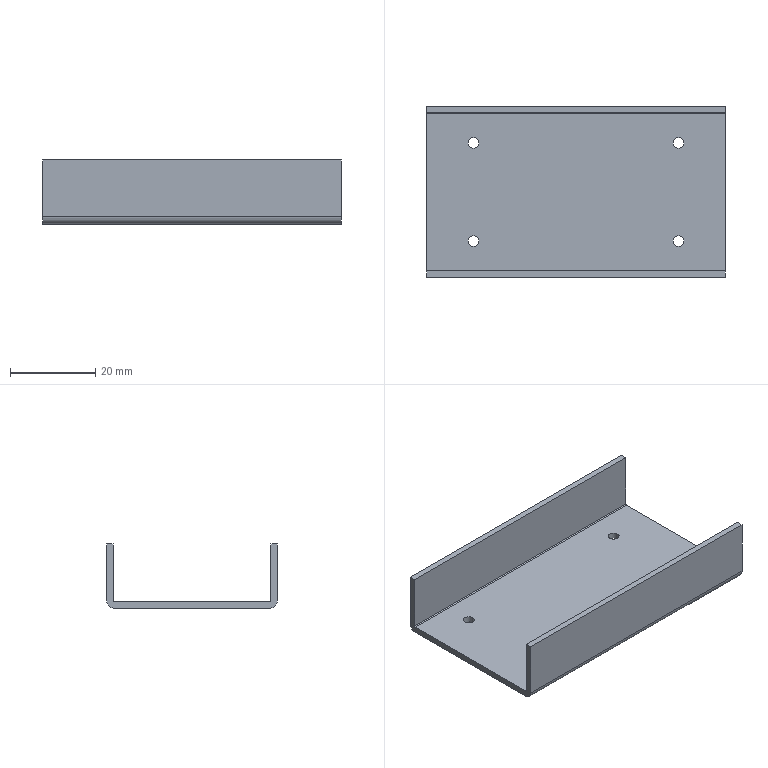Part | STEP file | FHD-021-014-B latch mounting seat | 1 solid | 18 faces | box 70 x 40 x 15 mm | volume 6920 mm3 | plane 10 | cylinder 8 | commonest cylinder face diameters 2.5 x4 0.4 x2 3.4 x2
STEP:
#1=CARTESIAN_POINT('',(0.,0.,0.));
#2=DIRECTION('',(0.,0.,1.));
#3=DIRECTION('',(1.,0.,0.));
#4=AXIS2_PLACEMENT_3D('',#1,#2,#3);
#5=CARTESIAN_POINT('',(35.,18.3,0.));
#6=VERTEX_POINT('',#5);
#7=CARTESIAN_POINT('',(35.,-18.3,0.));
#8=VERTEX_POINT('',#7);
#9=CARTESIAN_POINT('',(35.,0.,0.));
#10=DIRECTION('',(0.,-1.,0.));
#11=VECTOR('',#10,1.);
#12=LINE('',#9,#11);
#13=CARTESIAN_POINT('',(0.,0.,0.));
#14=DIRECTION('',(0.,0.,-1.));
#15=DIRECTION('',(-1.,0.,0.));
#16=AXIS2_PLACEMENT_3D('',#13,#14,#15);
#17=PLANE('',#16);
#18=CARTESIAN_POINT('',(-35.,0.));
#19=DIRECTION('',(0.,-1.));
#20=VECTOR('',#19,1.);
#21=LINE('',#18,#20);
#22=(GEOMETRIC_REPRESENTATION_CONTEXT(2)PARAMETRIC_REPRESENTATION_CONTEXT()REPRESENTATION_CONTEXT('',''));
#23=DEFINITIONAL_REPRESENTATION('',(#21),#22);
#24=PCURVE('',#17,#23);
#25=CARTESIAN_POINT('',(35.,-20.,-1.5));
#26=DIRECTION('',(1.,0.,0.));
#27=DIRECTION('',(0.,0.,-1.));
#28=AXIS2_PLACEMENT_3D('',#25,#26,#27);
#29=PLANE('',#28);
#30=CARTESIAN_POINT('',(-1.5,20.));
#31=DIRECTION('',(0.,-1.));
#32=VECTOR('',#31,1.);
#33=LINE('',#30,#32);
#34=(GEOMETRIC_REPRESENTATION_CONTEXT(2)PARAMETRIC_REPRESENTATION_CONTEXT()REPRESENTATION_CONTEXT('',''));
#35=DEFINITIONAL_REPRESENTATION('',(#33),#34);
#36=PCURVE('',#29,#35);
#37=SURFACE_CURVE('',#12,(#24,#36),.PCURVE_S1.);
#38=EDGE_CURVE('',#6,#8,#37,.T.);
#39=ORIENTED_EDGE('',*,*,#38,.F.);
#40=CARTESIAN_POINT('',(-35.,18.3,0.));
#41=VERTEX_POINT('',#40);
#42=CARTESIAN_POINT('',(0.,18.3,0.));
#43=DIRECTION('',(1.,0.,0.));
#44=VECTOR('',#43,1.);
#45=LINE('',#42,#44);
#46=CARTESIAN_POINT('',(0.,18.3));
#47=DIRECTION('',(-1.,0.));
#48=VECTOR('',#47,1.);
#49=LINE('',#46,#48);
#50=(GEOMETRIC_REPRESENTATION_CONTEXT(2)PARAMETRIC_REPRESENTATION_CONTEXT()REPRESENTATION_CONTEXT('',''));
#51=DEFINITIONAL_REPRESENTATION('',(#49),#50);
#52=PCURVE('',#17,#51);
#53=CARTESIAN_POINT('',(-35.,18.3,0.2));
#54=DIRECTION('',(-1.,0.,0.));
#55=DIRECTION('',(0.,0.,1.));
#56=AXIS2_PLACEMENT_3D('',#53,#54,#55);
#57=CYLINDRICAL_SURFACE('',#56,0.2);
#58=CARTESIAN_POINT('',(3.142,-35.));
#59=DIRECTION('',(0.,-1.));
#60=VECTOR('',#59,1.);
#61=LINE('',#58,#60);
#62=(GEOMETRIC_REPRESENTATION_CONTEXT(2)PARAMETRIC_REPRESENTATION_CONTEXT()REPRESENTATION_CONTEXT('',''));
#63=DEFINITIONAL_REPRESENTATION('',(#61),#62);
#64=PCURVE('',#57,#63);
#65=SURFACE_CURVE('',#45,(#52,#64),.PCURVE_S1.);
#66=EDGE_CURVE('',#41,#6,#65,.T.);
#67=ORIENTED_EDGE('',*,*,#66,.F.);
#68=CARTESIAN_POINT('',(-35.,-18.3,0.));
#69=VERTEX_POINT('',#68);
#70=CARTESIAN_POINT('',(-35.,0.,0.));
#71=DIRECTION('',(0.,1.,0.));
#72=VECTOR('',#71,1.);
#73=LINE('',#70,#72);
#74=CARTESIAN_POINT('',(35.,0.));
#75=DIRECTION('',(0.,1.));
#76=VECTOR('',#75,1.);
#77=LINE('',#74,#76);
#78=(GEOMETRIC_REPRESENTATION_CONTEXT(2)PARAMETRIC_REPRESENTATION_CONTEXT()REPRESENTATION_CONTEXT('',''));
#79=DEFINITIONAL_REPRESENTATION('',(#77),#78);
#80=PCURVE('',#17,#79);
#81=CARTESIAN_POINT('',(-35.,-20.,-1.5));
#82=DIRECTION('',(-1.,0.,0.));
#83=DIRECTION('',(0.,0.,1.));
#84=AXIS2_PLACEMENT_3D('',#81,#82,#83);
#85=PLANE('',#84);
#86=CARTESIAN_POINT('',(1.5,20.));
#87=DIRECTION('',(0.,1.));
#88=VECTOR('',#87,1.);
#89=LINE('',#86,#88);
#90=(GEOMETRIC_REPRESENTATION_CONTEXT(2)PARAMETRIC_REPRESENTATION_CONTEXT()REPRESENTATION_CONTEXT('',''));
#91=DEFINITIONAL_REPRESENTATION('',(#89),#90);
#92=PCURVE('',#85,#91);
#93=SURFACE_CURVE('',#73,(#80,#92),.PCURVE_S1.);
#94=EDGE_CURVE('',#69,#41,#93,.T.);
#95=ORIENTED_EDGE('',*,*,#94,.F.);
#96=CARTESIAN_POINT('',(0.,-18.3,0.));
#97=DIRECTION('',(-1.,0.,0.));
#98=VECTOR('',#97,1.);
#99=LINE('',#96,#98);
#100=CARTESIAN_POINT('',(0.,-18.3));
#101=DIRECTION('',(1.,0.));
#102=VECTOR('',#101,1.);
#103=LINE('',#100,#102);
#104=(GEOMETRIC_REPRESENTATION_CONTEXT(2)PARAMETRIC_REPRESENTATION_CONTEXT()REPRESENTATION_CONTEXT('',''));
#105=DEFINITIONAL_REPRESENTATION('',(#103),#104);
#106=PCURVE('',#17,#105);
#107=CARTESIAN_POINT('',(35.,-18.3,0.2));
#108=DIRECTION('',(1.,0.,0.));
#109=DIRECTION('',(0.,0.,-1.));
#110=AXIS2_PLACEMENT_3D('',#107,#108,#109);
#111=CYLINDRICAL_SURFACE('',#110,0.2);
#112=CARTESIAN_POINT('',(6.283,-35.));
#113=DIRECTION('',(0.,-1.));
#114=VECTOR('',#113,1.);
#115=LINE('',#112,#114);
#116=(GEOMETRIC_REPRESENTATION_CONTEXT(2)PARAMETRIC_REPRESENTATION_CONTEXT()REPRESENTATION_CONTEXT('',''));
#117=DEFINITIONAL_REPRESENTATION('',(#115),#116);
#118=PCURVE('',#111,#117);
#119=SURFACE_CURVE('',#99,(#106,#118),.PCURVE_S1.);
#120=EDGE_CURVE('',#8,#69,#119,.T.);
#121=ORIENTED_EDGE('',*,*,#120,.F.);
#122=EDGE_LOOP('',(#39,#67,#95,#121));
#123=FACE_BOUND('',#122,.T.);
#124=CARTESIAN_POINT('',(22.75,-11.5,0.));
#125=VERTEX_POINT('',#124);
#126=CARTESIAN_POINT('',(24.,-11.5,0.));
#127=DIRECTION('',(0.,0.,1.));
#128=DIRECTION('',(-1.,0.,0.));
#129=AXIS2_PLACEMENT_3D('',#126,#127,#128);
#130=CIRCLE('',#129,1.25);
#131=CARTESIAN_POINT('',(-22.75,-11.5));
#132=CARTESIAN_POINT('',(-22.75,-13.665));
#133=CARTESIAN_POINT('',(-24.625,-12.583));
#134=CARTESIAN_POINT('',(-26.5,-11.5));
#135=CARTESIAN_POINT('',(-24.625,-10.417));
#136=CARTESIAN_POINT('',(-22.75,-9.335));
#137=CARTESIAN_POINT('',(-22.75,-11.5));
#138=(BOUNDED_CURVE()B_SPLINE_CURVE(2,(#131,#132,#133,#134,#135,#136,#137),.UNSPECIFIED.,.T.,.F.)B_SPLINE_CURVE_WITH_KNOTS((1,2,2,2,2,1),(-2.094,0.,2.094,4.189,6.283,8.378),.UNSPECIFIED.)CURVE()GEOMETRIC_REPRESENTATION_ITEM()RATIONAL_B_SPLINE_CURVE((1.,0.5,1.,0.5,1.,0.5,1.))REPRESENTATION_ITEM(''));
#139=(GEOMETRIC_REPRESENTATION_CONTEXT(2)PARAMETRIC_REPRESENTATION_CONTEXT()REPRESENTATION_CONTEXT('',''));
#140=DEFINITIONAL_REPRESENTATION('',(#138),#139);
#141=PCURVE('',#17,#140);
#142=CARTESIAN_POINT('',(24.,-11.5,-1.5));
#143=DIRECTION('',(0.,0.,-1.));
#144=DIRECTION('',(-1.,0.,0.));
#145=AXIS2_PLACEMENT_3D('',#142,#143,#144);
#146=CYLINDRICAL_SURFACE('',#145,1.25);
#147=CARTESIAN_POINT('',(6.283,-1.5));
#148=DIRECTION('',(-1.,0.));
#149=VECTOR('',#148,1.);
#150=LINE('',#147,#149);
#151=(GEOMETRIC_REPRESENTATION_CONTEXT(2)PARAMETRIC_REPRESENTATION_CONTEXT()REPRESENTATION_CONTEXT('',''));
#152=DEFINITIONAL_REPRESENTATION('',(#150),#151);
#153=PCURVE('',#146,#152);
#154=SURFACE_CURVE('',#130,(#141,#153),.PCURVE_S1.);
#155=EDGE_CURVE('',#125,#125,#154,.T.);
#156=ORIENTED_EDGE('',*,*,#155,.F.);
#157=EDGE_LOOP('',(#156));
#158=FACE_BOUND('',#157,.T.);
#159=CARTESIAN_POINT('',(22.75,11.5,0.));
#160=VERTEX_POINT('',#159);
#161=CARTESIAN_POINT('',(24.,11.5,0.));
#162=DIRECTION('',(0.,0.,1.));
#163=DIRECTION('',(-1.,0.,0.));
#164=AXIS2_PLACEMENT_3D('',#161,#162,#163);
#165=CIRCLE('',#164,1.25);
#166=CARTESIAN_POINT('',(-22.75,11.5));
#167=CARTESIAN_POINT('',(-22.75,9.335));
#168=CARTESIAN_POINT('',(-24.625,10.417));
#169=CARTESIAN_POINT('',(-26.5,11.5));
#170=CARTESIAN_POINT('',(-24.625,12.583));
#171=CARTESIAN_POINT('',(-22.75,13.665));
#172=CARTESIAN_POINT('',(-22.75,11.5));
#173=(BOUNDED_CURVE()B_SPLINE_CURVE(2,(#166,#167,#168,#169,#170,#171,#172),.UNSPECIFIED.,.T.,.F.)B_SPLINE_CURVE_WITH_KNOTS((1,2,2,2,2,1),(-2.094,0.,2.094,4.189,6.283,8.378),.UNSPECIFIED.)CURVE()GEOMETRIC_REPRESENTATION_ITEM()RATIONAL_B_SPLINE_CURVE((1.,0.5,1.,0.5,1.,0.5,1.))REPRESENTATION_ITEM(''));
#174=(GEOMETRIC_REPRESENTATION_CONTEXT(2)PARAMETRIC_REPRESENTATION_CONTEXT()REPRESENTATION_CONTEXT('',''));
#175=DEFINITIONAL_REPRESENTATION('',(#173),#174);
#176=PCURVE('',#17,#175);
#177=CARTESIAN_POINT('',(24.,11.5,-1.5));
#178=DIRECTION('',(0.,0.,-1.));
#179=DIRECTION('',(-1.,0.,0.));
#180=AXIS2_PLACEMENT_3D('',#177,#178,#179);
#181=CYLINDRICAL_SURFACE('',#180,1.25);
#182=CARTESIAN_POINT('',(6.283,-1.5));
#183=DIRECTION('',(-1.,0.));
#184=VECTOR('',#183,1.);
#185=LINE('',#182,#184);
#186=(GEOMETRIC_REPRESENTATION_CONTEXT(2)PARAMETRIC_REPRESENTATION_CONTEXT()REPRESENTATION_CONTEXT('',''));
#187=DEFINITIONAL_REPRESENTATION('',(#185),#186);
#188=PCURVE('',#181,#187);
#189=SURFACE_CURVE('',#165,(#176,#188),.PCURVE_S1.);
#190=EDGE_CURVE('',#160,#160,#189,.T.);
#191=ORIENTED_EDGE('',*,*,#190,.F.);
#192=EDGE_LOOP('',(#191));
#193=FACE_BOUND('',#192,.T.);
#194=CARTESIAN_POINT('',(-25.25,11.5,0.));
#195=VERTEX_POINT('',#194);
#196=CARTESIAN_POINT('',(-24.,11.5,0.));
#197=DIRECTION('',(0.,0.,1.));
#198=DIRECTION('',(-1.,0.,0.));
#199=AXIS2_PLACEMENT_3D('',#196,#197,#198);
#200=CIRCLE('',#199,1.25);
#201=CARTESIAN_POINT('',(25.25,11.5));
#202=CARTESIAN_POINT('',(25.25,9.335));
#203=CARTESIAN_POINT('',(23.375,10.417));
#204=CARTESIAN_POINT('',(21.5,11.5));
#205=CARTESIAN_POINT('',(23.375,12.583));
#206=CARTESIAN_POINT('',(25.25,13.665));
#207=CARTESIAN_POINT('',(25.25,11.5));
#208=(BOUNDED_CURVE()B_SPLINE_CURVE(2,(#201,#202,#203,#204,#205,#206,#207),.UNSPECIFIED.,.T.,.F.)B_SPLINE_CURVE_WITH_KNOTS((1,2,2,2,2,1),(-2.094,0.,2.094,4.189,6.283,8.378),.UNSPECIFIED.)CURVE()GEOMETRIC_REPRESENTATION_ITEM()RATIONAL_B_SPLINE_CURVE((1.,0.5,1.,0.5,1.,0.5,1.))REPRESENTATION_ITEM(''));
#209=(GEOMETRIC_REPRESENTATION_CONTEXT(2)PARAMETRIC_REPRESENTATION_CONTEXT()REPRESENTATION_CONTEXT('',''));
#210=DEFINITIONAL_REPRESENTATION('',(#208),#209);
#211=PCURVE('',#17,#210);
#212=CARTESIAN_POINT('',(-24.,11.5,-1.5));
#213=DIRECTION('',(0.,0.,-1.));
#214=DIRECTION('',(-1.,0.,0.));
#215=AXIS2_PLACEMENT_3D('',#212,#213,#214);
#216=CYLINDRICAL_SURFACE('',#215,1.25);
#217=CARTESIAN_POINT('',(6.283,-1.5));
#218=DIRECTION('',(-1.,0.));
#219=VECTOR('',#218,1.);
#220=LINE('',#217,#219);
#221=(GEOMETRIC_REPRESENTATION_CONTEXT(2)PARAMETRIC_REPRESENTATION_CONTEXT()REPRESENTATION_CONTEXT('',''));
#222=DEFINITIONAL_REPRESENTATION('',(#220),#221);
#223=PCURVE('',#216,#222);
#224=SURFACE_CURVE('',#200,(#211,#223),.PCURVE_S1.);
#225=EDGE_CURVE('',#195,#195,#224,.T.);
#226=ORIENTED_EDGE('',*,*,#225,.F.);
#227=EDGE_LOOP('',(#226));
#228=FACE_BOUND('',#227,.T.);
#229=CARTESIAN_POINT('',(-25.25,-11.5,0.));
#230=VERTEX_POINT('',#229);
#231=CARTESIAN_POINT('',(-24.,-11.5,0.));
#232=DIRECTION('',(0.,0.,1.));
#233=DIRECTION('',(-1.,0.,0.));
#234=AXIS2_PLACEMENT_3D('',#231,#232,#233);
#235=CIRCLE('',#234,1.25);
#236=CARTESIAN_POINT('',(25.25,-11.5));
#237=CARTESIAN_POINT('',(25.25,-13.665));
#238=CARTESIAN_POINT('',(23.375,-12.583));
#239=CARTESIAN_POINT('',(21.5,-11.5));
#240=CARTESIAN_POINT('',(23.375,-10.417));
#241=CARTESIAN_POINT('',(25.25,-9.335));
#242=CARTESIAN_POINT('',(25.25,-11.5));
#243=(BOUNDED_CURVE()B_SPLINE_CURVE(2,(#236,#237,#238,#239,#240,#241,#242),.UNSPECIFIED.,.T.,.F.)B_SPLINE_CURVE_WITH_KNOTS((1,2,2,2,2,1),(-2.094,0.,2.094,4.189,6.283,8.378),.UNSPECIFIED.)CURVE()GEOMETRIC_REPRESENTATION_ITEM()RATIONAL_B_SPLINE_CURVE((1.,0.5,1.,0.5,1.,0.5,1.))REPRESENTATION_ITEM(''));
#244=(GEOMETRIC_REPRESENTATION_CONTEXT(2)PARAMETRIC_REPRESENTATION_CONTEXT()REPRESENTATION_CONTEXT('',''));
#245=DEFINITIONAL_REPRESENTATION('',(#243),#244);
#246=PCURVE('',#17,#245);
#247=CARTESIAN_POINT('',(-24.,-11.5,-1.5));
#248=DIRECTION('',(0.,0.,-1.));
#249=DIRECTION('',(-1.,0.,0.));
#250=AXIS2_PLACEMENT_3D('',#247,#248,#249);
#251=CYLINDRICAL_SURFACE('',#250,1.25);
#252=CARTESIAN_POINT('',(6.283,-1.5));
#253=DIRECTION('',(-1.,0.));
#254=VECTOR('',#253,1.);
#255=LINE('',#252,#254);
#256=(GEOMETRIC_REPRESENTATION_CONTEXT(2)PARAMETRIC_REPRESENTATION_CONTEXT()REPRESENTATION_CONTEXT('',''));
#257=DEFINITIONAL_REPRESENTATION('',(#255),#256);
#258=PCURVE('',#251,#257);
#259=SURFACE_CURVE('',#235,(#246,#258),.PCURVE_S1.);
#260=EDGE_CURVE('',#230,#230,#259,.T.);
#261=ORIENTED_EDGE('',*,*,#260,.F.);
#262=EDGE_LOOP('',(#261));
#263=FACE_BOUND('',#262,.T.);
#264=ADVANCED_FACE('',(#123,#158,#193,#228,#263),#17,.F.);
#265=ORIENTED_EDGE('',*,*,#120,.F.);
#266=CARTESIAN_POINT('',(35.,-18.5,0.2));
#267=VERTEX_POINT('',#266);
#268=CARTESIAN_POINT('',(35.,-18.3,0.2));
#269=DIRECTION('',(1.,0.,0.));
#270=DIRECTION('',(0.,0.,-1.));
#271=AXIS2_PLACEMENT_3D('',#268,#269,#270);
#272=CIRCLE('',#271,0.2);
#273=CARTESIAN_POINT('',(0.,0.));
#274=DIRECTION('',(1.,0.));
#275=VECTOR('',#274,1.);
#276=LINE('',#273,#275);
#277=(GEOMETRIC_REPRESENTATION_CONTEXT(2)PARAMETRIC_REPRESENTATION_CONTEXT()REPRESENTATION_CONTEXT('',''));
#278=DEFINITIONAL_REPRESENTATION('',(#276),#277);
#279=PCURVE('',#111,#278);
#280=CARTESIAN_POINT('',(-1.7,1.7));
#281=DIRECTION('',(1.,0.));
#282=AXIS2_PLACEMENT_2D('',#280,#281);
#283=CIRCLE('',#282,0.2);
#284=(GEOMETRIC_REPRESENTATION_CONTEXT(2)PARAMETRIC_REPRESENTATION_CONTEXT()REPRESENTATION_CONTEXT('',''));
#285=DEFINITIONAL_REPRESENTATION('',(#283),#284);
#286=PCURVE('',#29,#285);
#287=SURFACE_CURVE('',#272,(#279,#286),.PCURVE_S1.);
#288=EDGE_CURVE('',#267,#8,#287,.T.);
#289=ORIENTED_EDGE('',*,*,#288,.F.);
#290=CARTESIAN_POINT('',(-35.,-18.5,0.2));
#291=VERTEX_POINT('',#290);
#292=CARTESIAN_POINT('',(35.,-18.5,0.2));
#293=DIRECTION('',(-1.,0.,0.));
#294=VECTOR('',#293,1.);
#295=LINE('',#292,#294);
#296=CARTESIAN_POINT('',(4.712,0.));
#297=DIRECTION('',(0.,-1.));
#298=VECTOR('',#297,1.);
#299=LINE('',#296,#298);
#300=(GEOMETRIC_REPRESENTATION_CONTEXT(2)PARAMETRIC_REPRESENTATION_CONTEXT()REPRESENTATION_CONTEXT('',''));
#301=DEFINITIONAL_REPRESENTATION('',(#299),#300);
#302=PCURVE('',#111,#301);
#303=CARTESIAN_POINT('',(0.,-18.5,0.));
#304=DIRECTION('',(0.,1.,0.));
#305=DIRECTION('',(0.,0.,1.));
#306=AXIS2_PLACEMENT_3D('',#303,#304,#305);
#307=PLANE('',#306);
#308=CARTESIAN_POINT('',(0.2,35.));
#309=DIRECTION('',(0.,-1.));
#310=VECTOR('',#309,1.);
#311=LINE('',#308,#310);
#312=(GEOMETRIC_REPRESENTATION_CONTEXT(2)PARAMETRIC_REPRESENTATION_CONTEXT()REPRESENTATION_CONTEXT('',''));
#313=DEFINITIONAL_REPRESENTATION('',(#311),#312);
#314=PCURVE('',#307,#313);
#315=SURFACE_CURVE('',#295,(#302,#314),.PCURVE_S1.);
#316=EDGE_CURVE('',#267,#291,#315,.T.);
#317=ORIENTED_EDGE('',*,*,#316,.T.);
#318=CARTESIAN_POINT('',(-35.,-18.3,0.2));
#319=DIRECTION('',(1.,0.,0.));
#320=DIRECTION('',(0.,0.,-1.));
#321=AXIS2_PLACEMENT_3D('',#318,#319,#320);
#322=CIRCLE('',#321,0.2);
#323=CARTESIAN_POINT('',(0.,-70.));
#324=DIRECTION('',(1.,0.));
#325=VECTOR('',#324,1.);
#326=LINE('',#323,#325);
#327=(GEOMETRIC_REPRESENTATION_CONTEXT(2)PARAMETRIC_REPRESENTATION_CONTEXT()REPRESENTATION_CONTEXT('',''));
#328=DEFINITIONAL_REPRESENTATION('',(#326),#327);
#329=PCURVE('',#111,#328);
#330=CARTESIAN_POINT('',(1.5,1.7));
#331=CARTESIAN_POINT('',(1.5,2.046));
#332=CARTESIAN_POINT('',(1.8,1.873));
#333=CARTESIAN_POINT('',(2.1,1.7));
#334=CARTESIAN_POINT('',(1.8,1.527));
#335=CARTESIAN_POINT('',(1.5,1.354));
#336=CARTESIAN_POINT('',(1.5,1.7));
#337=(BOUNDED_CURVE()B_SPLINE_CURVE(2,(#330,#331,#332,#333,#334,#335,#336),.UNSPECIFIED.,.T.,.F.)B_SPLINE_CURVE_WITH_KNOTS((1,2,2,2,2,1),(-2.094,0.,2.094,4.189,6.283,8.378),.UNSPECIFIED.)CURVE()GEOMETRIC_REPRESENTATION_ITEM()RATIONAL_B_SPLINE_CURVE((1.,0.5,1.,0.5,1.,0.5,1.))REPRESENTATION_ITEM(''));
#338=(GEOMETRIC_REPRESENTATION_CONTEXT(2)PARAMETRIC_REPRESENTATION_CONTEXT()REPRESENTATION_CONTEXT('',''));
#339=DEFINITIONAL_REPRESENTATION('',(#337),#338);
#340=PCURVE('',#85,#339);
#341=SURFACE_CURVE('',#322,(#329,#340),.PCURVE_S1.);
#342=EDGE_CURVE('',#291,#69,#341,.T.);
#343=ORIENTED_EDGE('',*,*,#342,.T.);
#344=EDGE_LOOP('',(#265,#289,#317,#343));
#345=FACE_BOUND('',#344,.F.);
#346=ADVANCED_FACE('',(#345),#111,.F.);
#347=CARTESIAN_POINT('',(35.,-18.3,-1.5));
#348=VERTEX_POINT('',#347);
#349=CARTESIAN_POINT('',(35.,18.3,-1.5));
#350=VERTEX_POINT('',#349);
#351=CARTESIAN_POINT('',(35.,-20.,-1.5));
#352=DIRECTION('',(0.,1.,0.));
#353=VECTOR('',#352,1.);
#354=LINE('',#351,#353);
#355=CARTESIAN_POINT('',(0.,0.));
#356=DIRECTION('',(0.,1.));
#357=VECTOR('',#356,1.);
#358=LINE('',#355,#357);
#359=(GEOMETRIC_REPRESENTATION_CONTEXT(2)PARAMETRIC_REPRESENTATION_CONTEXT()REPRESENTATION_CONTEXT('',''));
#360=DEFINITIONAL_REPRESENTATION('',(#358),#359);
#361=PCURVE('',#29,#360);
#362=CARTESIAN_POINT('',(0.,0.,-1.5));
#363=DIRECTION('',(0.,0.,-1.));
#364=DIRECTION('',(-1.,0.,0.));
#365=AXIS2_PLACEMENT_3D('',#362,#363,#364);
#366=PLANE('',#365);
#367=CARTESIAN_POINT('',(-35.,-20.));
#368=DIRECTION('',(0.,1.));
#369=VECTOR('',#368,1.);
#370=LINE('',#367,#369);
#371=(GEOMETRIC_REPRESENTATION_CONTEXT(2)PARAMETRIC_REPRESENTATION_CONTEXT()REPRESENTATION_CONTEXT('',''));
#372=DEFINITIONAL_REPRESENTATION('',(#370),#371);
#373=PCURVE('',#366,#372);
#374=SURFACE_CURVE('',#354,(#361,#373),.PCURVE_S1.);
#375=EDGE_CURVE('',#348,#350,#374,.T.);
#376=ORIENTED_EDGE('',*,*,#375,.T.);
#377=CARTESIAN_POINT('',(35.,20.,0.2));
#378=VERTEX_POINT('',#377);
#379=CARTESIAN_POINT('',(35.,18.3,0.2));
#380=DIRECTION('',(-1.,0.,0.));
#381=DIRECTION('',(0.,0.,1.));
#382=AXIS2_PLACEMENT_3D('',#379,#380,#381);
#383=CIRCLE('',#382,1.7);
#384=CARTESIAN_POINT('',(-3.4,38.3));
#385=CARTESIAN_POINT('',(-3.4,41.244));
#386=CARTESIAN_POINT('',(-0.85,39.772));
#387=CARTESIAN_POINT('',(1.7,38.3));
#388=CARTESIAN_POINT('',(-0.85,36.828));
#389=CARTESIAN_POINT('',(-3.4,35.356));
#390=CARTESIAN_POINT('',(-3.4,38.3));
#391=(BOUNDED_CURVE()B_SPLINE_CURVE(2,(#384,#385,#386,#387,#388,#389,#390),.UNSPECIFIED.,.T.,.F.)B_SPLINE_CURVE_WITH_KNOTS((1,2,2,2,2,1),(-2.094,0.,2.094,4.189,6.283,8.378),.UNSPECIFIED.)CURVE()GEOMETRIC_REPRESENTATION_ITEM()RATIONAL_B_SPLINE_CURVE((1.,0.5,1.,0.5,1.,0.5,1.))REPRESENTATION_ITEM(''));
#392=(GEOMETRIC_REPRESENTATION_CONTEXT(2)PARAMETRIC_REPRESENTATION_CONTEXT()REPRESENTATION_CONTEXT('',''));
#393=DEFINITIONAL_REPRESENTATION('',(#391),#392);
#394=PCURVE('',#29,#393);
#395=CARTESIAN_POINT('',(-35.,18.3,0.2));
#396=DIRECTION('',(-1.,0.,0.));
#397=DIRECTION('',(0.,0.,1.));
#398=AXIS2_PLACEMENT_3D('',#395,#396,#397);
#399=CYLINDRICAL_SURFACE('',#398,1.7);
#400=CARTESIAN_POINT('',(0.,-70.));
#401=DIRECTION('',(1.,0.));
#402=VECTOR('',#401,1.);
#403=LINE('',#400,#402);
#404=(GEOMETRIC_REPRESENTATION_CONTEXT(2)PARAMETRIC_REPRESENTATION_CONTEXT()REPRESENTATION_CONTEXT('',''));
#405=DEFINITIONAL_REPRESENTATION('',(#403),#404);
#406=PCURVE('',#399,#405);
#407=SURFACE_CURVE('',#383,(#394,#406),.PCURVE_S1.);
#408=EDGE_CURVE('',#378,#350,#407,.T.);
#409=ORIENTED_EDGE('',*,*,#408,.F.);
#410=CARTESIAN_POINT('',(35.,20.,13.5));
#411=VERTEX_POINT('',#410);
#412=CARTESIAN_POINT('',(35.,20.,0.));
#413=DIRECTION('',(0.,0.,-1.));
#414=VECTOR('',#413,1.);
#415=LINE('',#412,#414);
#416=CARTESIAN_POINT('',(-1.5,40.));
#417=DIRECTION('',(1.,0.));
#418=VECTOR('',#417,1.);
#419=LINE('',#416,#418);
#420=(GEOMETRIC_REPRESENTATION_CONTEXT(2)PARAMETRIC_REPRESENTATION_CONTEXT()REPRESENTATION_CONTEXT('',''));
#421=DEFINITIONAL_REPRESENTATION('',(#419),#420);
#422=PCURVE('',#29,#421);
#423=CARTESIAN_POINT('',(0.,20.,0.));
#424=DIRECTION('',(0.,-1.,0.));
#425=DIRECTION('',(0.,0.,-1.));
#426=AXIS2_PLACEMENT_3D('',#423,#424,#425);
#427=PLANE('',#426);
#428=CARTESIAN_POINT('',(0.,35.));
#429=DIRECTION('',(1.,0.));
#430=VECTOR('',#429,1.);
#431=LINE('',#428,#430);
#432=(GEOMETRIC_REPRESENTATION_CONTEXT(2)PARAMETRIC_REPRESENTATION_CONTEXT()REPRESENTATION_CONTEXT('',''));
#433=DEFINITIONAL_REPRESENTATION('',(#431),#432);
#434=PCURVE('',#427,#433);
#435=SURFACE_CURVE('',#415,(#422,#434),.PCURVE_S1.);
#436=EDGE_CURVE('',#411,#378,#435,.T.);
#437=ORIENTED_EDGE('',*,*,#436,.F.);
#438=CARTESIAN_POINT('',(35.,18.5,13.5));
#439=VERTEX_POINT('',#438);
#440=CARTESIAN_POINT('',(35.,20.,13.5));
#441=DIRECTION('',(0.,-1.,0.));
#442=VECTOR('',#441,1.);
#443=LINE('',#440,#442);
#444=CARTESIAN_POINT('',(-15.,40.));
#445=DIRECTION('',(0.,-1.));
#446=VECTOR('',#445,1.);
#447=LINE('',#444,#446);
#448=(GEOMETRIC_REPRESENTATION_CONTEXT(2)PARAMETRIC_REPRESENTATION_CONTEXT()REPRESENTATION_CONTEXT('',''));
#449=DEFINITIONAL_REPRESENTATION('',(#447),#448);
#450=PCURVE('',#29,#449);
#451=CARTESIAN_POINT('',(35.,20.,13.5));
#452=DIRECTION('',(0.,0.,-1.));
#453=DIRECTION('',(0.,1.,0.));
#454=AXIS2_PLACEMENT_3D('',#451,#452,#453);
#455=PLANE('',#454);
#456=CARTESIAN_POINT('',(0.,0.));
#457=DIRECTION('',(-1.,0.));
#458=VECTOR('',#457,1.);
#459=LINE('',#456,#458);
#460=(GEOMETRIC_REPRESENTATION_CONTEXT(2)PARAMETRIC_REPRESENTATION_CONTEXT()REPRESENTATION_CONTEXT('',''));
#461=DEFINITIONAL_REPRESENTATION('',(#459),#460);
#462=PCURVE('',#455,#461);
#463=SURFACE_CURVE('',#443,(#450,#462),.PCURVE_S1.);
#464=EDGE_CURVE('',#411,#439,#463,.T.);
#465=ORIENTED_EDGE('',*,*,#464,.T.);
#466=CARTESIAN_POINT('',(35.,18.5,0.2));
#467=VERTEX_POINT('',#466);
#468=CARTESIAN_POINT('',(35.,18.5,0.));
#469=DIRECTION('',(0.,0.,1.));
#470=VECTOR('',#469,1.);
#471=LINE('',#468,#470);
#472=CARTESIAN_POINT('',(-1.5,38.5));
#473=DIRECTION('',(-1.,0.));
#474=VECTOR('',#473,1.);
#475=LINE('',#472,#474);
#476=(GEOMETRIC_REPRESENTATION_CONTEXT(2)PARAMETRIC_REPRESENTATION_CONTEXT()REPRESENTATION_CONTEXT('',''));
#477=DEFINITIONAL_REPRESENTATION('',(#475),#476);
#478=PCURVE('',#29,#477);
#479=CARTESIAN_POINT('',(0.,18.5,0.));
#480=DIRECTION('',(0.,-1.,0.));
#481=DIRECTION('',(0.,0.,-1.));
#482=AXIS2_PLACEMENT_3D('',#479,#480,#481);
#483=PLANE('',#482);
#484=CARTESIAN_POINT('',(0.,35.));
#485=DIRECTION('',(-1.,0.));
#486=VECTOR('',#485,1.);
#487=LINE('',#484,#486);
#488=(GEOMETRIC_REPRESENTATION_CONTEXT(2)PARAMETRIC_REPRESENTATION_CONTEXT()REPRESENTATION_CONTEXT('',''));
#489=DEFINITIONAL_REPRESENTATION('',(#487),#488);
#490=PCURVE('',#483,#489);
#491=SURFACE_CURVE('',#471,(#478,#490),.PCURVE_S1.);
#492=EDGE_CURVE('',#467,#439,#491,.T.);
#493=ORIENTED_EDGE('',*,*,#492,.F.);
#494=CARTESIAN_POINT('',(35.,18.3,0.2));
#495=DIRECTION('',(-1.,0.,0.));
#496=DIRECTION('',(0.,0.,1.));
#497=AXIS2_PLACEMENT_3D('',#494,#495,#496);
#498=CIRCLE('',#497,0.2);
#499=CARTESIAN_POINT('',(-1.9,38.3));
#500=CARTESIAN_POINT('',(-1.9,38.646));
#501=CARTESIAN_POINT('',(-1.6,38.473));
#502=CARTESIAN_POINT('',(-1.3,38.3));
#503=CARTESIAN_POINT('',(-1.6,38.127));
#504=CARTESIAN_POINT('',(-1.9,37.954));
#505=CARTESIAN_POINT('',(-1.9,38.3));
#506=(BOUNDED_CURVE()B_SPLINE_CURVE(2,(#499,#500,#501,#502,#503,#504,#505),.UNSPECIFIED.,.T.,.F.)B_SPLINE_CURVE_WITH_KNOTS((1,2,2,2,2,1),(-2.094,0.,2.094,4.189,6.283,8.378),.UNSPECIFIED.)CURVE()GEOMETRIC_REPRESENTATION_ITEM()RATIONAL_B_SPLINE_CURVE((1.,0.5,1.,0.5,1.,0.5,1.))REPRESENTATION_ITEM(''));
#507=(GEOMETRIC_REPRESENTATION_CONTEXT(2)PARAMETRIC_REPRESENTATION_CONTEXT()REPRESENTATION_CONTEXT('',''));
#508=DEFINITIONAL_REPRESENTATION('',(#506),#507);
#509=PCURVE('',#29,#508);
#510=CARTESIAN_POINT('',(0.,-70.));
#511=DIRECTION('',(1.,0.));
#512=VECTOR('',#511,1.);
#513=LINE('',#510,#512);
#514=(GEOMETRIC_REPRESENTATION_CONTEXT(2)PARAMETRIC_REPRESENTATION_CONTEXT()REPRESENTATION_CONTEXT('',''));
#515=DEFINITIONAL_REPRESENTATION('',(#513),#514);
#516=PCURVE('',#57,#515);
#517=SURFACE_CURVE('',#498,(#509,#516),.PCURVE_S1.);
#518=EDGE_CURVE('',#467,#6,#517,.T.);
#519=ORIENTED_EDGE('',*,*,#518,.T.);
#520=ORIENTED_EDGE('',*,*,#38,.T.);
#521=ORIENTED_EDGE('',*,*,#288,.F.);
#522=CARTESIAN_POINT('',(35.,-18.5,13.5));
#523=VERTEX_POINT('',#522);
#524=CARTESIAN_POINT('',(35.,-18.5,0.));
#525=DIRECTION('',(0.,0.,-1.));
#526=VECTOR('',#525,1.);
#527=LINE('',#524,#526);
#528=CARTESIAN_POINT('',(-1.5,1.5));
#529=DIRECTION('',(1.,0.));
#530=VECTOR('',#529,1.);
#531=LINE('',#528,#530);
#532=(GEOMETRIC_REPRESENTATION_CONTEXT(2)PARAMETRIC_REPRESENTATION_CONTEXT()REPRESENTATION_CONTEXT('',''));
#533=DEFINITIONAL_REPRESENTATION('',(#531),#532);
#534=PCURVE('',#29,#533);
#535=CARTESIAN_POINT('',(0.,35.));
#536=DIRECTION('',(-1.,0.));
#537=VECTOR('',#536,1.);
#538=LINE('',#535,#537);
#539=(GEOMETRIC_REPRESENTATION_CONTEXT(2)PARAMETRIC_REPRESENTATION_CONTEXT()REPRESENTATION_CONTEXT('',''));
#540=DEFINITIONAL_REPRESENTATION('',(#538),#539);
#541=PCURVE('',#307,#540);
#542=SURFACE_CURVE('',#527,(#534,#541),.PCURVE_S1.);
#543=EDGE_CURVE('',#523,#267,#542,.T.);
#544=ORIENTED_EDGE('',*,*,#543,.F.);
#545=CARTESIAN_POINT('',(35.,-20.,13.5));
#546=VERTEX_POINT('',#545);
#547=CARTESIAN_POINT('',(35.,-20.,13.5));
#548=DIRECTION('',(0.,-1.,0.));
#549=VECTOR('',#548,1.);
#550=LINE('',#547,#549);
#551=CARTESIAN_POINT('',(-15.,0.));
#552=DIRECTION('',(0.,-1.));
#553=VECTOR('',#552,1.);
#554=LINE('',#551,#553);
#555=(GEOMETRIC_REPRESENTATION_CONTEXT(2)PARAMETRIC_REPRESENTATION_CONTEXT()REPRESENTATION_CONTEXT('',''));
#556=DEFINITIONAL_REPRESENTATION('',(#554),#555);
#557=PCURVE('',#29,#556);
#558=CARTESIAN_POINT('',(-35.,-20.,13.5));
#559=DIRECTION('',(0.,0.,-1.));
#560=DIRECTION('',(0.,1.,0.));
#561=AXIS2_PLACEMENT_3D('',#558,#559,#560);
#562=PLANE('',#561);
#563=CARTESIAN_POINT('',(0.,70.));
#564=DIRECTION('',(-1.,0.));
#565=VECTOR('',#564,1.);
#566=LINE('',#563,#565);
#567=(GEOMETRIC_REPRESENTATION_CONTEXT(2)PARAMETRIC_REPRESENTATION_CONTEXT()REPRESENTATION_CONTEXT('',''));
#568=DEFINITIONAL_REPRESENTATION('',(#566),#567);
#569=PCURVE('',#562,#568);
#570=SURFACE_CURVE('',#550,(#557,#569),.PCURVE_S1.);
#571=EDGE_CURVE('',#523,#546,#570,.T.);
#572=ORIENTED_EDGE('',*,*,#571,.T.);
#573=CARTESIAN_POINT('',(35.,-20.,0.2));
#574=VERTEX_POINT('',#573);
#575=CARTESIAN_POINT('',(35.,-20.,13.5));
#576=DIRECTION('',(0.,0.,1.));
#577=VECTOR('',#576,1.);
#578=LINE('',#575,#577);
#579=CARTESIAN_POINT('',(-15.,0.));
#580=DIRECTION('',(-1.,0.));
#581=VECTOR('',#580,1.);
#582=LINE('',#579,#581);
#583=(GEOMETRIC_REPRESENTATION_CONTEXT(2)PARAMETRIC_REPRESENTATION_CONTEXT()REPRESENTATION_CONTEXT('',''));
#584=DEFINITIONAL_REPRESENTATION('',(#582),#583);
#585=PCURVE('',#29,#584);
#586=CARTESIAN_POINT('',(0.,-20.,0.));
#587=DIRECTION('',(0.,1.,0.));
#588=DIRECTION('',(0.,0.,1.));
#589=AXIS2_PLACEMENT_3D('',#586,#587,#588);
#590=PLANE('',#589);
#591=CARTESIAN_POINT('',(13.5,35.));
#592=DIRECTION('',(1.,0.));
#593=VECTOR('',#592,1.);
#594=LINE('',#591,#593);
#595=(GEOMETRIC_REPRESENTATION_CONTEXT(2)PARAMETRIC_REPRESENTATION_CONTEXT()REPRESENTATION_CONTEXT('',''));
#596=DEFINITIONAL_REPRESENTATION('',(#594),#595);
#597=PCURVE('',#590,#596);
#598=SURFACE_CURVE('',#578,(#585,#597),.PCURVE_S1.);
#599=EDGE_CURVE('',#574,#546,#598,.T.);
#600=ORIENTED_EDGE('',*,*,#599,.F.);
#601=CARTESIAN_POINT('',(35.,-18.3,0.2));
#602=DIRECTION('',(-1.,0.,0.));
#603=DIRECTION('',(0.,0.,-1.));
#604=AXIS2_PLACEMENT_3D('',#601,#602,#603);
#605=CIRCLE('',#604,1.7);
#606=CARTESIAN_POINT('',(0.,1.7));
#607=CARTESIAN_POINT('',(0.,-1.244));
#608=CARTESIAN_POINT('',(-2.55,0.2278));
#609=CARTESIAN_POINT('',(-5.1,1.7));
#610=CARTESIAN_POINT('',(-2.55,3.172));
#611=CARTESIAN_POINT('',(0.,4.644));
#612=CARTESIAN_POINT('',(0.,1.7));
#613=(BOUNDED_CURVE()B_SPLINE_CURVE(2,(#606,#607,#608,#609,#610,#611,#612),.UNSPECIFIED.,.T.,.F.)B_SPLINE_CURVE_WITH_KNOTS((1,2,2,2,2,1),(-2.094,0.,2.094,4.189,6.283,8.378),.UNSPECIFIED.)CURVE()GEOMETRIC_REPRESENTATION_ITEM()RATIONAL_B_SPLINE_CURVE((1.,0.5,1.,0.5,1.,0.5,1.))REPRESENTATION_ITEM(''));
#614=(GEOMETRIC_REPRESENTATION_CONTEXT(2)PARAMETRIC_REPRESENTATION_CONTEXT()REPRESENTATION_CONTEXT('',''));
#615=DEFINITIONAL_REPRESENTATION('',(#613),#614);
#616=PCURVE('',#29,#615);
#617=CARTESIAN_POINT('',(35.,-18.3,0.2));
#618=DIRECTION('',(1.,0.,0.));
#619=DIRECTION('',(0.,0.,-1.));
#620=AXIS2_PLACEMENT_3D('',#617,#618,#619);
#621=CYLINDRICAL_SURFACE('',#620,1.7);
#622=CARTESIAN_POINT('',(6.283,0.));
#623=DIRECTION('',(-1.,0.));
#624=VECTOR('',#623,1.);
#625=LINE('',#622,#624);
#626=(GEOMETRIC_REPRESENTATION_CONTEXT(2)PARAMETRIC_REPRESENTATION_CONTEXT()REPRESENTATION_CONTEXT('',''));
#627=DEFINITIONAL_REPRESENTATION('',(#625),#626);
#628=PCURVE('',#621,#627);
#629=SURFACE_CURVE('',#605,(#616,#628),.PCURVE_S1.);
#630=EDGE_CURVE('',#348,#574,#629,.T.);
#631=ORIENTED_EDGE('',*,*,#630,.F.);
#632=EDGE_LOOP('',(#376,#409,#437,#465,#493,#519,#520,#521,#544,#572,#600,#631));
#633=FACE_BOUND('',#632,.T.);
#634=ADVANCED_FACE('',(#633),#29,.T.);
#635=ORIENTED_EDGE('',*,*,#66,.F.);
#636=CARTESIAN_POINT('',(-35.,18.5,0.2));
#637=VERTEX_POINT('',#636);
#638=CARTESIAN_POINT('',(-35.,18.3,0.2));
#639=DIRECTION('',(-1.,0.,0.));
#640=DIRECTION('',(0.,0.,1.));
#641=AXIS2_PLACEMENT_3D('',#638,#639,#640);
#642=CIRCLE('',#641,0.2);
#643=CARTESIAN_POINT('',(0.,0.));
#644=DIRECTION('',(1.,0.));
#645=VECTOR('',#644,1.);
#646=LINE('',#643,#645);
#647=(GEOMETRIC_REPRESENTATION_CONTEXT(2)PARAMETRIC_REPRESENTATION_CONTEXT()REPRESENTATION_CONTEXT('',''));
#648=DEFINITIONAL_REPRESENTATION('',(#646),#647);
#649=PCURVE('',#57,#648);
#650=CARTESIAN_POINT('',(1.7,38.3));
#651=DIRECTION('',(1.,0.));
#652=AXIS2_PLACEMENT_2D('',#650,#651);
#653=CIRCLE('',#652,0.2);
#654=(GEOMETRIC_REPRESENTATION_CONTEXT(2)PARAMETRIC_REPRESENTATION_CONTEXT()REPRESENTATION_CONTEXT('',''));
#655=DEFINITIONAL_REPRESENTATION('',(#653),#654);
#656=PCURVE('',#85,#655);
#657=SURFACE_CURVE('',#642,(#649,#656),.PCURVE_S1.);
#658=EDGE_CURVE('',#637,#41,#657,.T.);
#659=ORIENTED_EDGE('',*,*,#658,.F.);
#660=CARTESIAN_POINT('',(-35.,18.5,0.2));
#661=DIRECTION('',(1.,0.,0.));
#662=VECTOR('',#661,1.);
#663=LINE('',#660,#662);
#664=CARTESIAN_POINT('',(1.571,0.));
#665=DIRECTION('',(0.,-1.));
#666=VECTOR('',#665,1.);
#667=LINE('',#664,#666);
#668=(GEOMETRIC_REPRESENTATION_CONTEXT(2)PARAMETRIC_REPRESENTATION_CONTEXT()REPRESENTATION_CONTEXT('',''));
#669=DEFINITIONAL_REPRESENTATION('',(#667),#668);
#670=PCURVE('',#57,#669);
#671=CARTESIAN_POINT('',(-0.2,-35.));
#672=DIRECTION('',(0.,1.));
#673=VECTOR('',#672,1.);
#674=LINE('',#671,#673);
#675=(GEOMETRIC_REPRESENTATION_CONTEXT(2)PARAMETRIC_REPRESENTATION_CONTEXT()REPRESENTATION_CONTEXT('',''));
#676=DEFINITIONAL_REPRESENTATION('',(#674),#675);
#677=PCURVE('',#483,#676);
#678=SURFACE_CURVE('',#663,(#670,#677),.PCURVE_S1.);
#679=EDGE_CURVE('',#637,#467,#678,.T.);
#680=ORIENTED_EDGE('',*,*,#679,.T.);
#681=ORIENTED_EDGE('',*,*,#518,.T.);
#682=EDGE_LOOP('',(#635,#659,#680,#681));
#683=FACE_BOUND('',#682,.F.);
#684=ADVANCED_FACE('',(#683),#57,.F.);
#685=ORIENTED_EDGE('',*,*,#94,.T.);
#686=ORIENTED_EDGE('',*,*,#658,.F.);
#687=CARTESIAN_POINT('',(-35.,18.5,13.5));
#688=VERTEX_POINT('',#687);
#689=CARTESIAN_POINT('',(-35.,18.5,0.));
#690=DIRECTION('',(0.,0.,-1.));
#691=VECTOR('',#690,1.);
#692=LINE('',#689,#691);
#693=CARTESIAN_POINT('',(1.5,38.5));
#694=DIRECTION('',(-1.,0.));
#695=VECTOR('',#694,1.);
#696=LINE('',#693,#695);
#697=(GEOMETRIC_REPRESENTATION_CONTEXT(2)PARAMETRIC_REPRESENTATION_CONTEXT()REPRESENTATION_CONTEXT('',''));
#698=DEFINITIONAL_REPRESENTATION('',(#696),#697);
#699=PCURVE('',#85,#698);
#700=CARTESIAN_POINT('',(0.,-35.));
#701=DIRECTION('',(1.,0.));
#702=VECTOR('',#701,1.);
#703=LINE('',#700,#702);
#704=(GEOMETRIC_REPRESENTATION_CONTEXT(2)PARAMETRIC_REPRESENTATION_CONTEXT()REPRESENTATION_CONTEXT('',''));
#705=DEFINITIONAL_REPRESENTATION('',(#703),#704);
#706=PCURVE('',#483,#705);
#707=SURFACE_CURVE('',#692,(#699,#706),.PCURVE_S1.);
#708=EDGE_CURVE('',#688,#637,#707,.T.);
#709=ORIENTED_EDGE('',*,*,#708,.F.);
#710=CARTESIAN_POINT('',(-35.,20.,13.5));
#711=VERTEX_POINT('',#710);
#712=CARTESIAN_POINT('',(-35.,20.,13.5));
#713=DIRECTION('',(0.,1.,0.));
#714=VECTOR('',#713,1.);
#715=LINE('',#712,#714);
#716=CARTESIAN_POINT('',(15.,40.));
#717=DIRECTION('',(0.,1.));
#718=VECTOR('',#717,1.);
#719=LINE('',#716,#718);
#720=(GEOMETRIC_REPRESENTATION_CONTEXT(2)PARAMETRIC_REPRESENTATION_CONTEXT()REPRESENTATION_CONTEXT('',''));
#721=DEFINITIONAL_REPRESENTATION('',(#719),#720);
#722=PCURVE('',#85,#721);
#723=CARTESIAN_POINT('',(0.,-70.));
#724=DIRECTION('',(1.,0.));
#725=VECTOR('',#724,1.);
#726=LINE('',#723,#725);
#727=(GEOMETRIC_REPRESENTATION_CONTEXT(2)PARAMETRIC_REPRESENTATION_CONTEXT()REPRESENTATION_CONTEXT('',''));
#728=DEFINITIONAL_REPRESENTATION('',(#726),#727);
#729=PCURVE('',#455,#728);
#730=SURFACE_CURVE('',#715,(#722,#729),.PCURVE_S1.);
#731=EDGE_CURVE('',#688,#711,#730,.T.);
#732=ORIENTED_EDGE('',*,*,#731,.T.);
#733=CARTESIAN_POINT('',(-35.,20.,0.2));
#734=VERTEX_POINT('',#733);
#735=CARTESIAN_POINT('',(-35.,20.,13.5));
#736=DIRECTION('',(0.,0.,1.));
#737=VECTOR('',#736,1.);
#738=LINE('',#735,#737);
#739=CARTESIAN_POINT('',(15.,40.));
#740=DIRECTION('',(1.,0.));
#741=VECTOR('',#740,1.);
#742=LINE('',#739,#741);
#743=(GEOMETRIC_REPRESENTATION_CONTEXT(2)PARAMETRIC_REPRESENTATION_CONTEXT()REPRESENTATION_CONTEXT('',''));
#744=DEFINITIONAL_REPRESENTATION('',(#742),#743);
#745=PCURVE('',#85,#744);
#746=CARTESIAN_POINT('',(-13.5,-35.));
#747=DIRECTION('',(-1.,0.));
#748=VECTOR('',#747,1.);
#749=LINE('',#746,#748);
#750=(GEOMETRIC_REPRESENTATION_CONTEXT(2)PARAMETRIC_REPRESENTATION_CONTEXT()REPRESENTATION_CONTEXT('',''));
#751=DEFINITIONAL_REPRESENTATION('',(#749),#750);
#752=PCURVE('',#427,#751);
#753=SURFACE_CURVE('',#738,(#745,#752),.PCURVE_S1.);
#754=EDGE_CURVE('',#734,#711,#753,.T.);
#755=ORIENTED_EDGE('',*,*,#754,.F.);
#756=CARTESIAN_POINT('',(-35.,18.3,-1.5));
#757=VERTEX_POINT('',#756);
#758=CARTESIAN_POINT('',(-35.,18.3,0.2));
#759=DIRECTION('',(1.,0.,0.));
#760=DIRECTION('',(0.,0.,1.));
#761=AXIS2_PLACEMENT_3D('',#758,#759,#760);
#762=CIRCLE('',#761,1.7);
#763=CARTESIAN_POINT('',(3.4,38.3));
#764=CARTESIAN_POINT('',(3.4,35.356));
#765=CARTESIAN_POINT('',(0.85,36.828));
#766=CARTESIAN_POINT('',(-1.7,38.3));
#767=CARTESIAN_POINT('',(0.85,39.772));
#768=CARTESIAN_POINT('',(3.4,41.244));
#769=CARTESIAN_POINT('',(3.4,38.3));
#770=(BOUNDED_CURVE()B_SPLINE_CURVE(2,(#763,#764,#765,#766,#767,#768,#769),.UNSPECIFIED.,.T.,.F.)B_SPLINE_CURVE_WITH_KNOTS((1,2,2,2,2,1),(-2.094,0.,2.094,4.189,6.283,8.378),.UNSPECIFIED.)CURVE()GEOMETRIC_REPRESENTATION_ITEM()RATIONAL_B_SPLINE_CURVE((1.,0.5,1.,0.5,1.,0.5,1.))REPRESENTATION_ITEM(''));
#771=(GEOMETRIC_REPRESENTATION_CONTEXT(2)PARAMETRIC_REPRESENTATION_CONTEXT()REPRESENTATION_CONTEXT('',''));
#772=DEFINITIONAL_REPRESENTATION('',(#770),#771);
#773=PCURVE('',#85,#772);
#774=CARTESIAN_POINT('',(6.283,0.));
#775=DIRECTION('',(-1.,0.));
#776=VECTOR('',#775,1.);
#777=LINE('',#774,#776);
#778=(GEOMETRIC_REPRESENTATION_CONTEXT(2)PARAMETRIC_REPRESENTATION_CONTEXT()REPRESENTATION_CONTEXT('',''));
#779=DEFINITIONAL_REPRESENTATION('',(#777),#778);
#780=PCURVE('',#399,#779);
#781=SURFACE_CURVE('',#762,(#773,#780),.PCURVE_S1.);
#782=EDGE_CURVE('',#757,#734,#781,.T.);
#783=ORIENTED_EDGE('',*,*,#782,.F.);
#784=CARTESIAN_POINT('',(-35.,-18.3,-1.5));
#785=VERTEX_POINT('',#784);
#786=CARTESIAN_POINT('',(-35.,-20.,-1.5));
#787=DIRECTION('',(0.,-1.,0.));
#788=VECTOR('',#787,1.);
#789=LINE('',#786,#788);
#790=CARTESIAN_POINT('',(0.,0.));
#791=DIRECTION('',(0.,-1.));
#792=VECTOR('',#791,1.);
#793=LINE('',#790,#792);
#794=(GEOMETRIC_REPRESENTATION_CONTEXT(2)PARAMETRIC_REPRESENTATION_CONTEXT()REPRESENTATION_CONTEXT('',''));
#795=DEFINITIONAL_REPRESENTATION('',(#793),#794);
#796=PCURVE('',#85,#795);
#797=CARTESIAN_POINT('',(35.,-20.));
#798=DIRECTION('',(0.,-1.));
#799=VECTOR('',#798,1.);
#800=LINE('',#797,#799);
#801=(GEOMETRIC_REPRESENTATION_CONTEXT(2)PARAMETRIC_REPRESENTATION_CONTEXT()REPRESENTATION_CONTEXT('',''));
#802=DEFINITIONAL_REPRESENTATION('',(#800),#801);
#803=PCURVE('',#366,#802);
#804=SURFACE_CURVE('',#789,(#796,#803),.PCURVE_S1.);
#805=EDGE_CURVE('',#757,#785,#804,.T.);
#806=ORIENTED_EDGE('',*,*,#805,.T.);
#807=CARTESIAN_POINT('',(-35.,-20.,0.2));
#808=VERTEX_POINT('',#807);
#809=CARTESIAN_POINT('',(-35.,-18.3,0.2));
#810=DIRECTION('',(1.,0.,0.));
#811=DIRECTION('',(0.,0.,-1.));
#812=AXIS2_PLACEMENT_3D('',#809,#810,#811);
#813=CIRCLE('',#812,1.7);
#814=CARTESIAN_POINT('',(0.,1.7));
#815=CARTESIAN_POINT('',(0.,4.644));
#816=CARTESIAN_POINT('',(2.55,3.172));
#817=CARTESIAN_POINT('',(5.1,1.7));
#818=CARTESIAN_POINT('',(2.55,0.2278));
#819=CARTESIAN_POINT('',(0.,-1.244));
#820=CARTESIAN_POINT('',(0.,1.7));
#821=(BOUNDED_CURVE()B_SPLINE_CURVE(2,(#814,#815,#816,#817,#818,#819,#820),.UNSPECIFIED.,.T.,.F.)B_SPLINE_CURVE_WITH_KNOTS((1,2,2,2,2,1),(-2.094,0.,2.094,4.189,6.283,8.378),.UNSPECIFIED.)CURVE()GEOMETRIC_REPRESENTATION_ITEM()RATIONAL_B_SPLINE_CURVE((1.,0.5,1.,0.5,1.,0.5,1.))REPRESENTATION_ITEM(''));
#822=(GEOMETRIC_REPRESENTATION_CONTEXT(2)PARAMETRIC_REPRESENTATION_CONTEXT()REPRESENTATION_CONTEXT('',''));
#823=DEFINITIONAL_REPRESENTATION('',(#821),#822);
#824=PCURVE('',#85,#823);
#825=CARTESIAN_POINT('',(0.,-70.));
#826=DIRECTION('',(1.,0.));
#827=VECTOR('',#826,1.);
#828=LINE('',#825,#827);
#829=(GEOMETRIC_REPRESENTATION_CONTEXT(2)PARAMETRIC_REPRESENTATION_CONTEXT()REPRESENTATION_CONTEXT('',''));
#830=DEFINITIONAL_REPRESENTATION('',(#828),#829);
#831=PCURVE('',#621,#830);
#832=SURFACE_CURVE('',#813,(#824,#831),.PCURVE_S1.);
#833=EDGE_CURVE('',#808,#785,#832,.T.);
#834=ORIENTED_EDGE('',*,*,#833,.F.);
#835=CARTESIAN_POINT('',(-35.,-20.,13.5));
#836=VERTEX_POINT('',#835);
#837=CARTESIAN_POINT('',(-35.,-20.,0.));
#838=DIRECTION('',(0.,0.,-1.));
#839=VECTOR('',#838,1.);
#840=LINE('',#837,#839);
#841=CARTESIAN_POINT('',(1.5,0.));
#842=DIRECTION('',(-1.,0.));
#843=VECTOR('',#842,1.);
#844=LINE('',#841,#843);
#845=(GEOMETRIC_REPRESENTATION_CONTEXT(2)PARAMETRIC_REPRESENTATION_CONTEXT()REPRESENTATION_CONTEXT('',''));
#846=DEFINITIONAL_REPRESENTATION('',(#844),#845);
#847=PCURVE('',#85,#846);
#848=CARTESIAN_POINT('',(0.,-35.));
#849=DIRECTION('',(-1.,0.));
#850=VECTOR('',#849,1.);
#851=LINE('',#848,#850);
#852=(GEOMETRIC_REPRESENTATION_CONTEXT(2)PARAMETRIC_REPRESENTATION_CONTEXT()REPRESENTATION_CONTEXT('',''));
#853=DEFINITIONAL_REPRESENTATION('',(#851),#852);
#854=PCURVE('',#590,#853);
#855=SURFACE_CURVE('',#840,(#847,#854),.PCURVE_S1.);
#856=EDGE_CURVE('',#836,#808,#855,.T.);
#857=ORIENTED_EDGE('',*,*,#856,.F.);
#858=CARTESIAN_POINT('',(-35.,-18.5,13.5));
#859=VERTEX_POINT('',#858);
#860=CARTESIAN_POINT('',(-35.,-20.,13.5));
#861=DIRECTION('',(0.,1.,0.));
#862=VECTOR('',#861,1.);
#863=LINE('',#860,#862);
#864=CARTESIAN_POINT('',(15.,0.));
#865=DIRECTION('',(0.,1.));
#866=VECTOR('',#865,1.);
#867=LINE('',#864,#866);
#868=(GEOMETRIC_REPRESENTATION_CONTEXT(2)PARAMETRIC_REPRESENTATION_CONTEXT()REPRESENTATION_CONTEXT('',''));
#869=DEFINITIONAL_REPRESENTATION('',(#867),#868);
#870=PCURVE('',#85,#869);
#871=CARTESIAN_POINT('',(0.,0.));
#872=DIRECTION('',(1.,0.));
#873=VECTOR('',#872,1.);
#874=LINE('',#871,#873);
#875=(GEOMETRIC_REPRESENTATION_CONTEXT(2)PARAMETRIC_REPRESENTATION_CONTEXT()REPRESENTATION_CONTEXT('',''));
#876=DEFINITIONAL_REPRESENTATION('',(#874),#875);
#877=PCURVE('',#562,#876);
#878=SURFACE_CURVE('',#863,(#870,#877),.PCURVE_S1.);
#879=EDGE_CURVE('',#836,#859,#878,.T.);
#880=ORIENTED_EDGE('',*,*,#879,.T.);
#881=CARTESIAN_POINT('',(-35.,-18.5,0.));
#882=DIRECTION('',(0.,0.,1.));
#883=VECTOR('',#882,1.);
#884=LINE('',#881,#883);
#885=CARTESIAN_POINT('',(1.5,1.5));
#886=DIRECTION('',(1.,0.));
#887=VECTOR('',#886,1.);
#888=LINE('',#885,#887);
#889=(GEOMETRIC_REPRESENTATION_CONTEXT(2)PARAMETRIC_REPRESENTATION_CONTEXT()REPRESENTATION_CONTEXT('',''));
#890=DEFINITIONAL_REPRESENTATION('',(#888),#889);
#891=PCURVE('',#85,#890);
#892=CARTESIAN_POINT('',(0.,-35.));
#893=DIRECTION('',(1.,0.));
#894=VECTOR('',#893,1.);
#895=LINE('',#892,#894);
#896=(GEOMETRIC_REPRESENTATION_CONTEXT(2)PARAMETRIC_REPRESENTATION_CONTEXT()REPRESENTATION_CONTEXT('',''));
#897=DEFINITIONAL_REPRESENTATION('',(#895),#896);
#898=PCURVE('',#307,#897);
#899=SURFACE_CURVE('',#884,(#891,#898),.PCURVE_S1.);
#900=EDGE_CURVE('',#291,#859,#899,.T.);
#901=ORIENTED_EDGE('',*,*,#900,.F.);
#902=ORIENTED_EDGE('',*,*,#342,.T.);
#903=EDGE_LOOP('',(#685,#686,#709,#732,#755,#783,#806,#834,#857,#880,#901,#902));
#904=FACE_BOUND('',#903,.T.);
#905=ADVANCED_FACE('',(#904),#85,.T.);
#906=ORIENTED_EDGE('',*,*,#155,.F.);
#907=CARTESIAN_POINT('',(22.75,-11.5,-1.5));
#908=VERTEX_POINT('',#907);
#909=CARTESIAN_POINT('',(22.75,-11.5,0.));
#910=CARTESIAN_POINT('',(22.75,-11.5,-1.5));
#911=B_SPLINE_CURVE_WITH_KNOTS('',1,(#909,#910),.UNSPECIFIED.,.F.,.F.,(2,2),(-1.5,0.),.PIECEWISE_BEZIER_KNOTS.);
#912=CARTESIAN_POINT('',(6.283,0.));
#913=DIRECTION('',(0.,1.));
#914=VECTOR('',#913,1.);
#915=LINE('',#912,#914);
#916=(GEOMETRIC_REPRESENTATION_CONTEXT(2)PARAMETRIC_REPRESENTATION_CONTEXT()REPRESENTATION_CONTEXT('',''));
#917=DEFINITIONAL_REPRESENTATION('',(#915),#916);
#918=PCURVE('',#146,#917);
#919=CARTESIAN_POINT('',(0.,0.));
#920=DIRECTION('',(0.,1.));
#921=VECTOR('',#920,1.);
#922=LINE('',#919,#921);
#923=(GEOMETRIC_REPRESENTATION_CONTEXT(2)PARAMETRIC_REPRESENTATION_CONTEXT()REPRESENTATION_CONTEXT('',''));
#924=DEFINITIONAL_REPRESENTATION('',(#922),#923);
#925=PCURVE('',#146,#924);
#926=SEAM_CURVE('',#911,(#918,#925),.PCURVE_S1.);
#927=EDGE_CURVE('',#125,#908,#926,.T.);
#928=ORIENTED_EDGE('',*,*,#927,.T.);
#929=CARTESIAN_POINT('',(24.,-11.5,-1.5));
#930=DIRECTION('',(0.,0.,1.));
#931=DIRECTION('',(-1.,0.,0.));
#932=AXIS2_PLACEMENT_3D('',#929,#930,#931);
#933=CIRCLE('',#932,1.25);
#934=CARTESIAN_POINT('',(6.283,0.));
#935=DIRECTION('',(-1.,0.));
#936=VECTOR('',#935,1.);
#937=LINE('',#934,#936);
#938=(GEOMETRIC_REPRESENTATION_CONTEXT(2)PARAMETRIC_REPRESENTATION_CONTEXT()REPRESENTATION_CONTEXT('',''));
#939=DEFINITIONAL_REPRESENTATION('',(#937),#938);
#940=PCURVE('',#146,#939);
#941=CARTESIAN_POINT('',(-22.75,-11.5));
#942=CARTESIAN_POINT('',(-22.75,-13.665));
#943=CARTESIAN_POINT('',(-24.625,-12.583));
#944=CARTESIAN_POINT('',(-26.5,-11.5));
#945=CARTESIAN_POINT('',(-24.625,-10.417));
#946=CARTESIAN_POINT('',(-22.75,-9.335));
#947=CARTESIAN_POINT('',(-22.75,-11.5));
#948=(BOUNDED_CURVE()B_SPLINE_CURVE(2,(#941,#942,#943,#944,#945,#946,#947),.UNSPECIFIED.,.T.,.F.)B_SPLINE_CURVE_WITH_KNOTS((1,2,2,2,2,1),(-2.094,0.,2.094,4.189,6.283,8.378),.UNSPECIFIED.)CURVE()GEOMETRIC_REPRESENTATION_ITEM()RATIONAL_B_SPLINE_CURVE((1.,0.5,1.,0.5,1.,0.5,1.))REPRESENTATION_ITEM(''));
#949=(GEOMETRIC_REPRESENTATION_CONTEXT(2)PARAMETRIC_REPRESENTATION_CONTEXT()REPRESENTATION_CONTEXT('',''));
#950=DEFINITIONAL_REPRESENTATION('',(#948),#949);
#951=PCURVE('',#366,#950);
#952=SURFACE_CURVE('',#933,(#940,#951),.PCURVE_S1.);
#953=EDGE_CURVE('',#908,#908,#952,.T.);
#954=ORIENTED_EDGE('',*,*,#953,.T.);
#955=ORIENTED_EDGE('',*,*,#927,.F.);
#956=EDGE_LOOP('',(#906,#928,#954,#955));
#957=FACE_BOUND('',#956,.F.);
#958=ADVANCED_FACE('',(#957),#146,.F.);
#959=ORIENTED_EDGE('',*,*,#190,.F.);
#960=CARTESIAN_POINT('',(22.75,11.5,-1.5));
#961=VERTEX_POINT('',#960);
#962=CARTESIAN_POINT('',(22.75,11.5,0.));
#963=CARTESIAN_POINT('',(22.75,11.5,-1.5));
#964=B_SPLINE_CURVE_WITH_KNOTS('',1,(#962,#963),.UNSPECIFIED.,.F.,.F.,(2,2),(-1.5,0.),.PIECEWISE_BEZIER_KNOTS.);
#965=CARTESIAN_POINT('',(6.283,0.));
#966=DIRECTION('',(0.,1.));
#967=VECTOR('',#966,1.);
#968=LINE('',#965,#967);
#969=(GEOMETRIC_REPRESENTATION_CONTEXT(2)PARAMETRIC_REPRESENTATION_CONTEXT()REPRESENTATION_CONTEXT('',''));
#970=DEFINITIONAL_REPRESENTATION('',(#968),#969);
#971=PCURVE('',#181,#970);
#972=CARTESIAN_POINT('',(0.,0.));
#973=DIRECTION('',(0.,1.));
#974=VECTOR('',#973,1.);
#975=LINE('',#972,#974);
#976=(GEOMETRIC_REPRESENTATION_CONTEXT(2)PARAMETRIC_REPRESENTATION_CONTEXT()REPRESENTATION_CONTEXT('',''));
#977=DEFINITIONAL_REPRESENTATION('',(#975),#976);
#978=PCURVE('',#181,#977);
#979=SEAM_CURVE('',#964,(#971,#978),.PCURVE_S1.);
#980=EDGE_CURVE('',#160,#961,#979,.T.);
#981=ORIENTED_EDGE('',*,*,#980,.T.);
#982=CARTESIAN_POINT('',(24.,11.5,-1.5));
#983=DIRECTION('',(0.,0.,1.));
#984=DIRECTION('',(-1.,0.,0.));
#985=AXIS2_PLACEMENT_3D('',#982,#983,#984);
#986=CIRCLE('',#985,1.25);
#987=CARTESIAN_POINT('',(6.283,0.));
#988=DIRECTION('',(-1.,0.));
#989=VECTOR('',#988,1.);
#990=LINE('',#987,#989);
#991=(GEOMETRIC_REPRESENTATION_CONTEXT(2)PARAMETRIC_REPRESENTATION_CONTEXT()REPRESENTATION_CONTEXT('',''));
#992=DEFINITIONAL_REPRESENTATION('',(#990),#991);
#993=PCURVE('',#181,#992);
#994=CARTESIAN_POINT('',(-22.75,11.5));
#995=CARTESIAN_POINT('',(-22.75,9.335));
#996=CARTESIAN_POINT('',(-24.625,10.417));
#997=CARTESIAN_POINT('',(-26.5,11.5));
#998=CARTESIAN_POINT('',(-24.625,12.583));
#999=CARTESIAN_POINT('',(-22.75,13.665));
#1000=CARTESIAN_POINT('',(-22.75,11.5));
#1001=(BOUNDED_CURVE()B_SPLINE_CURVE(2,(#994,#995,#996,#997,#998,#999,#1000),.UNSPECIFIED.,.T.,.F.)B_SPLINE_CURVE_WITH_KNOTS((1,2,2,2,2,1),(-2.094,0.,2.094,4.189,6.283,8.378),.UNSPECIFIED.)CURVE()GEOMETRIC_REPRESENTATION_ITEM()RATIONAL_B_SPLINE_CURVE((1.,0.5,1.,0.5,1.,0.5,1.))REPRESENTATION_ITEM(''));
#1002=(GEOMETRIC_REPRESENTATION_CONTEXT(2)PARAMETRIC_REPRESENTATION_CONTEXT()REPRESENTATION_CONTEXT('',''));
#1003=DEFINITIONAL_REPRESENTATION('',(#1001),#1002);
#1004=PCURVE('',#366,#1003);
#1005=SURFACE_CURVE('',#986,(#993,#1004),.PCURVE_S1.);
#1006=EDGE_CURVE('',#961,#961,#1005,.T.);
#1007=ORIENTED_EDGE('',*,*,#1006,.T.);
#1008=ORIENTED_EDGE('',*,*,#980,.F.);
#1009=EDGE_LOOP('',(#959,#981,#1007,#1008));
#1010=FACE_BOUND('',#1009,.F.);
#1011=ADVANCED_FACE('',(#1010),#181,.F.);
#1012=ORIENTED_EDGE('',*,*,#225,.F.);
#1013=CARTESIAN_POINT('',(-25.25,11.5,-1.5));
#1014=VERTEX_POINT('',#1013);
#1015=CARTESIAN_POINT('',(-25.25,11.5,0.));
#1016=CARTESIAN_POINT('',(-25.25,11.5,-1.5));
#1017=B_SPLINE_CURVE_WITH_KNOTS('',1,(#1015,#1016),.UNSPECIFIED.,.F.,.F.,(2,2),(-1.5,0.),.PIECEWISE_BEZIER_KNOTS.);
#1018=CARTESIAN_POINT('',(6.283,0.));
#1019=DIRECTION('',(0.,1.));
#1020=VECTOR('',#1019,1.);
#1021=LINE('',#1018,#1020);
#1022=(GEOMETRIC_REPRESENTATION_CONTEXT(2)PARAMETRIC_REPRESENTATION_CONTEXT()REPRESENTATION_CONTEXT('',''));
#1023=DEFINITIONAL_REPRESENTATION('',(#1021),#1022);
#1024=PCURVE('',#216,#1023);
#1025=CARTESIAN_POINT('',(0.,0.));
#1026=DIRECTION('',(0.,1.));
#1027=VECTOR('',#1026,1.);
#1028=LINE('',#1025,#1027);
#1029=(GEOMETRIC_REPRESENTATION_CONTEXT(2)PARAMETRIC_REPRESENTATION_CONTEXT()REPRESENTATION_CONTEXT('',''));
#1030=DEFINITIONAL_REPRESENTATION('',(#1028),#1029);
#1031=PCURVE('',#216,#1030);
#1032=SEAM_CURVE('',#1017,(#1024,#1031),.PCURVE_S1.);
#1033=EDGE_CURVE('',#195,#1014,#1032,.T.);
#1034=ORIENTED_EDGE('',*,*,#1033,.T.);
#1035=CARTESIAN_POINT('',(-24.,11.5,-1.5));
#1036=DIRECTION('',(0.,0.,1.));
#1037=DIRECTION('',(-1.,0.,0.));
#1038=AXIS2_PLACEMENT_3D('',#1035,#1036,#1037);
#1039=CIRCLE('',#1038,1.25);
#1040=CARTESIAN_POINT('',(6.283,0.));
#1041=DIRECTION('',(-1.,0.));
#1042=VECTOR('',#1041,1.);
#1043=LINE('',#1040,#1042);
#1044=(GEOMETRIC_REPRESENTATION_CONTEXT(2)PARAMETRIC_REPRESENTATION_CONTEXT()REPRESENTATION_CONTEXT('',''));
#1045=DEFINITIONAL_REPRESENTATION('',(#1043),#1044);
#1046=PCURVE('',#216,#1045);
#1047=CARTESIAN_POINT('',(25.25,11.5));
#1048=CARTESIAN_POINT('',(25.25,9.335));
#1049=CARTESIAN_POINT('',(23.375,10.417));
#1050=CARTESIAN_POINT('',(21.5,11.5));
#1051=CARTESIAN_POINT('',(23.375,12.583));
#1052=CARTESIAN_POINT('',(25.25,13.665));
#1053=CARTESIAN_POINT('',(25.25,11.5));
#1054=(BOUNDED_CURVE()B_SPLINE_CURVE(2,(#1047,#1048,#1049,#1050,#1051,#1052,#1053),.UNSPECIFIED.,.T.,.F.)B_SPLINE_CURVE_WITH_KNOTS((1,2,2,2,2,1),(-2.094,0.,2.094,4.189,6.283,8.378),.UNSPECIFIED.)CURVE()GEOMETRIC_REPRESENTATION_ITEM()RATIONAL_B_SPLINE_CURVE((1.,0.5,1.,0.5,1.,0.5,1.))REPRESENTATION_ITEM(''));
#1055=(GEOMETRIC_REPRESENTATION_CONTEXT(2)PARAMETRIC_REPRESENTATION_CONTEXT()REPRESENTATION_CONTEXT('',''));
#1056=DEFINITIONAL_REPRESENTATION('',(#1054),#1055);
#1057=PCURVE('',#366,#1056);
#1058=SURFACE_CURVE('',#1039,(#1046,#1057),.PCURVE_S1.);
#1059=EDGE_CURVE('',#1014,#1014,#1058,.T.);
#1060=ORIENTED_EDGE('',*,*,#1059,.T.);
#1061=ORIENTED_EDGE('',*,*,#1033,.F.);
#1062=EDGE_LOOP('',(#1012,#1034,#1060,#1061));
#1063=FACE_BOUND('',#1062,.F.);
#1064=ADVANCED_FACE('',(#1063),#216,.F.);
#1065=ORIENTED_EDGE('',*,*,#260,.F.);
#1066=CARTESIAN_POINT('',(-25.25,-11.5,-1.5));
#1067=VERTEX_POINT('',#1066);
#1068=CARTESIAN_POINT('',(-25.25,-11.5,0.));
#1069=CARTESIAN_POINT('',(-25.25,-11.5,-1.5));
#1070=B_SPLINE_CURVE_WITH_KNOTS('',1,(#1068,#1069),.UNSPECIFIED.,.F.,.F.,(2,2),(-1.5,0.),.PIECEWISE_BEZIER_KNOTS.);
#1071=CARTESIAN_POINT('',(6.283,0.));
#1072=DIRECTION('',(0.,1.));
#1073=VECTOR('',#1072,1.);
#1074=LINE('',#1071,#1073);
#1075=(GEOMETRIC_REPRESENTATION_CONTEXT(2)PARAMETRIC_REPRESENTATION_CONTEXT()REPRESENTATION_CONTEXT('',''));
#1076=DEFINITIONAL_REPRESENTATION('',(#1074),#1075);
#1077=PCURVE('',#251,#1076);
#1078=CARTESIAN_POINT('',(0.,0.));
#1079=DIRECTION('',(0.,1.));
#1080=VECTOR('',#1079,1.);
#1081=LINE('',#1078,#1080);
#1082=(GEOMETRIC_REPRESENTATION_CONTEXT(2)PARAMETRIC_REPRESENTATION_CONTEXT()REPRESENTATION_CONTEXT('',''));
#1083=DEFINITIONAL_REPRESENTATION('',(#1081),#1082);
#1084=PCURVE('',#251,#1083);
#1085=SEAM_CURVE('',#1070,(#1077,#1084),.PCURVE_S1.);
#1086=EDGE_CURVE('',#230,#1067,#1085,.T.);
#1087=ORIENTED_EDGE('',*,*,#1086,.T.);
#1088=CARTESIAN_POINT('',(-24.,-11.5,-1.5));
#1089=DIRECTION('',(0.,0.,1.));
#1090=DIRECTION('',(-1.,0.,0.));
#1091=AXIS2_PLACEMENT_3D('',#1088,#1089,#1090);
#1092=CIRCLE('',#1091,1.25);
#1093=CARTESIAN_POINT('',(6.283,0.));
#1094=DIRECTION('',(-1.,0.));
#1095=VECTOR('',#1094,1.);
#1096=LINE('',#1093,#1095);
#1097=(GEOMETRIC_REPRESENTATION_CONTEXT(2)PARAMETRIC_REPRESENTATION_CONTEXT()REPRESENTATION_CONTEXT('',''));
#1098=DEFINITIONAL_REPRESENTATION('',(#1096),#1097);
#1099=PCURVE('',#251,#1098);
#1100=CARTESIAN_POINT('',(25.25,-11.5));
#1101=CARTESIAN_POINT('',(25.25,-13.665));
#1102=CARTESIAN_POINT('',(23.375,-12.583));
#1103=CARTESIAN_POINT('',(21.5,-11.5));
#1104=CARTESIAN_POINT('',(23.375,-10.417));
#1105=CARTESIAN_POINT('',(25.25,-9.335));
#1106=CARTESIAN_POINT('',(25.25,-11.5));
#1107=(BOUNDED_CURVE()B_SPLINE_CURVE(2,(#1100,#1101,#1102,#1103,#1104,#1105,#1106),.UNSPECIFIED.,.T.,.F.)B_SPLINE_CURVE_WITH_KNOTS((1,2,2,2,2,1),(-2.094,0.,2.094,4.189,6.283,8.378),.UNSPECIFIED.)CURVE()GEOMETRIC_REPRESENTATION_ITEM()RATIONAL_B_SPLINE_CURVE((1.,0.5,1.,0.5,1.,0.5,1.))REPRESENTATION_ITEM(''));
#1108=(GEOMETRIC_REPRESENTATION_CONTEXT(2)PARAMETRIC_REPRESENTATION_CONTEXT()REPRESENTATION_CONTEXT('',''));
#1109=DEFINITIONAL_REPRESENTATION('',(#1107),#1108);
#1110=PCURVE('',#366,#1109);
#1111=SURFACE_CURVE('',#1092,(#1099,#1110),.PCURVE_S1.);
#1112=EDGE_CURVE('',#1067,#1067,#1111,.T.);
#1113=ORIENTED_EDGE('',*,*,#1112,.T.);
#1114=ORIENTED_EDGE('',*,*,#1086,.F.);
#1115=EDGE_LOOP('',(#1065,#1087,#1113,#1114));
#1116=FACE_BOUND('',#1115,.F.);
#1117=ADVANCED_FACE('',(#1116),#251,.F.);
#1118=ORIENTED_EDGE('',*,*,#900,.T.);
#1119=CARTESIAN_POINT('',(0.,-18.5,13.5));
#1120=DIRECTION('',(1.,0.,0.));
#1121=VECTOR('',#1120,1.);
#1122=LINE('',#1119,#1121);
#1123=CARTESIAN_POINT('',(13.5,0.));
#1124=DIRECTION('',(0.,1.));
#1125=VECTOR('',#1124,1.);
#1126=LINE('',#1123,#1125);
#1127=(GEOMETRIC_REPRESENTATION_CONTEXT(2)PARAMETRIC_REPRESENTATION_CONTEXT()REPRESENTATION_CONTEXT('',''));
#1128=DEFINITIONAL_REPRESENTATION('',(#1126),#1127);
#1129=PCURVE('',#307,#1128);
#1130=CARTESIAN_POINT('',(1.5,35.));
#1131=DIRECTION('',(0.,1.));
#1132=VECTOR('',#1131,1.);
#1133=LINE('',#1130,#1132);
#1134=(GEOMETRIC_REPRESENTATION_CONTEXT(2)PARAMETRIC_REPRESENTATION_CONTEXT()REPRESENTATION_CONTEXT('',''));
#1135=DEFINITIONAL_REPRESENTATION('',(#1133),#1134);
#1136=PCURVE('',#562,#1135);
#1137=SURFACE_CURVE('',#1122,(#1129,#1136),.PCURVE_S1.);
#1138=EDGE_CURVE('',#859,#523,#1137,.T.);
#1139=ORIENTED_EDGE('',*,*,#1138,.T.);
#1140=ORIENTED_EDGE('',*,*,#543,.T.);
#1141=ORIENTED_EDGE('',*,*,#316,.T.);
#1142=EDGE_LOOP('',(#1118,#1139,#1140,#1141));
#1143=FACE_BOUND('',#1142,.T.);
#1144=ADVANCED_FACE('',(#1143),#307,.T.);
#1145=ORIENTED_EDGE('',*,*,#805,.F.);
#1146=CARTESIAN_POINT('',(0.,18.3,-1.5));
#1147=DIRECTION('',(1.,0.,0.));
#1148=VECTOR('',#1147,1.);
#1149=LINE('',#1146,#1148);
#1150=CARTESIAN_POINT('',(0.,18.3));
#1151=DIRECTION('',(-1.,0.));
#1152=VECTOR('',#1151,1.);
#1153=LINE('',#1150,#1152);
#1154=(GEOMETRIC_REPRESENTATION_CONTEXT(2)PARAMETRIC_REPRESENTATION_CONTEXT()REPRESENTATION_CONTEXT('',''));
#1155=DEFINITIONAL_REPRESENTATION('',(#1153),#1154);
#1156=PCURVE('',#366,#1155);
#1157=CARTESIAN_POINT('',(3.142,-35.));
#1158=DIRECTION('',(0.,-1.));
#1159=VECTOR('',#1158,1.);
#1160=LINE('',#1157,#1159);
#1161=(GEOMETRIC_REPRESENTATION_CONTEXT(2)PARAMETRIC_REPRESENTATION_CONTEXT()REPRESENTATION_CONTEXT('',''));
#1162=DEFINITIONAL_REPRESENTATION('',(#1160),#1161);
#1163=PCURVE('',#399,#1162);
#1164=SURFACE_CURVE('',#1149,(#1156,#1163),.PCURVE_S1.);
#1165=EDGE_CURVE('',#757,#350,#1164,.T.);
#1166=ORIENTED_EDGE('',*,*,#1165,.T.);
#1167=ORIENTED_EDGE('',*,*,#375,.F.);
#1168=CARTESIAN_POINT('',(0.,-18.3,-1.5));
#1169=DIRECTION('',(-1.,0.,0.));
#1170=VECTOR('',#1169,1.);
#1171=LINE('',#1168,#1170);
#1172=CARTESIAN_POINT('',(0.,-18.3));
#1173=DIRECTION('',(1.,0.));
#1174=VECTOR('',#1173,1.);
#1175=LINE('',#1172,#1174);
#1176=(GEOMETRIC_REPRESENTATION_CONTEXT(2)PARAMETRIC_REPRESENTATION_CONTEXT()REPRESENTATION_CONTEXT('',''));
#1177=DEFINITIONAL_REPRESENTATION('',(#1175),#1176);
#1178=PCURVE('',#366,#1177);
#1179=CARTESIAN_POINT('',(6.283,-35.));
#1180=DIRECTION('',(0.,-1.));
#1181=VECTOR('',#1180,1.);
#1182=LINE('',#1179,#1181);
#1183=(GEOMETRIC_REPRESENTATION_CONTEXT(2)PARAMETRIC_REPRESENTATION_CONTEXT()REPRESENTATION_CONTEXT('',''));
#1184=DEFINITIONAL_REPRESENTATION('',(#1182),#1183);
#1185=PCURVE('',#621,#1184);
#1186=SURFACE_CURVE('',#1171,(#1178,#1185),.PCURVE_S1.);
#1187=EDGE_CURVE('',#348,#785,#1186,.T.);
#1188=ORIENTED_EDGE('',*,*,#1187,.T.);
#1189=EDGE_LOOP('',(#1145,#1166,#1167,#1188));
#1190=FACE_BOUND('',#1189,.T.);
#1191=ORIENTED_EDGE('',*,*,#953,.T.);
#1192=EDGE_LOOP('',(#1191));
#1193=FACE_BOUND('',#1192,.T.);
#1194=ORIENTED_EDGE('',*,*,#1006,.T.);
#1195=EDGE_LOOP('',(#1194));
#1196=FACE_BOUND('',#1195,.T.);
#1197=ORIENTED_EDGE('',*,*,#1059,.T.);
#1198=EDGE_LOOP('',(#1197));
#1199=FACE_BOUND('',#1198,.T.);
#1200=ORIENTED_EDGE('',*,*,#1112,.T.);
#1201=EDGE_LOOP('',(#1200));
#1202=FACE_BOUND('',#1201,.T.);
#1203=ADVANCED_FACE('',(#1190,#1193,#1196,#1199,#1202),#366,.T.);
#1204=ORIENTED_EDGE('',*,*,#492,.T.);
#1205=CARTESIAN_POINT('',(0.,18.5,13.5));
#1206=DIRECTION('',(-1.,0.,0.));
#1207=VECTOR('',#1206,1.);
#1208=LINE('',#1205,#1207);
#1209=CARTESIAN_POINT('',(-13.5,0.));
#1210=DIRECTION('',(0.,-1.));
#1211=VECTOR('',#1210,1.);
#1212=LINE('',#1209,#1211);
#1213=(GEOMETRIC_REPRESENTATION_CONTEXT(2)PARAMETRIC_REPRESENTATION_CONTEXT()REPRESENTATION_CONTEXT('',''));
#1214=DEFINITIONAL_REPRESENTATION('',(#1212),#1213);
#1215=PCURVE('',#483,#1214);
#1216=CARTESIAN_POINT('',(-1.5,-35.));
#1217=DIRECTION('',(0.,-1.));
#1218=VECTOR('',#1217,1.);
#1219=LINE('',#1216,#1218);
#1220=(GEOMETRIC_REPRESENTATION_CONTEXT(2)PARAMETRIC_REPRESENTATION_CONTEXT()REPRESENTATION_CONTEXT('',''));
#1221=DEFINITIONAL_REPRESENTATION('',(#1219),#1220);
#1222=PCURVE('',#455,#1221);
#1223=SURFACE_CURVE('',#1208,(#1215,#1222),.PCURVE_S1.);
#1224=EDGE_CURVE('',#439,#688,#1223,.T.);
#1225=ORIENTED_EDGE('',*,*,#1224,.T.);
#1226=ORIENTED_EDGE('',*,*,#708,.T.);
#1227=ORIENTED_EDGE('',*,*,#679,.T.);
#1228=EDGE_LOOP('',(#1204,#1225,#1226,#1227));
#1229=FACE_BOUND('',#1228,.T.);
#1230=ADVANCED_FACE('',(#1229),#483,.T.);
#1231=ORIENTED_EDGE('',*,*,#879,.F.);
#1232=CARTESIAN_POINT('',(-35.,-20.,13.5));
#1233=DIRECTION('',(-1.,0.,0.));
#1234=VECTOR('',#1233,1.);
#1235=LINE('',#1232,#1234);
#1236=CARTESIAN_POINT('',(0.,0.));
#1237=DIRECTION('',(0.,-1.));
#1238=VECTOR('',#1237,1.);
#1239=LINE('',#1236,#1238);
#1240=(GEOMETRIC_REPRESENTATION_CONTEXT(2)PARAMETRIC_REPRESENTATION_CONTEXT()REPRESENTATION_CONTEXT('',''));
#1241=DEFINITIONAL_REPRESENTATION('',(#1239),#1240);
#1242=PCURVE('',#562,#1241);
#1243=CARTESIAN_POINT('',(13.5,-35.));
#1244=DIRECTION('',(0.,-1.));
#1245=VECTOR('',#1244,1.);
#1246=LINE('',#1243,#1245);
#1247=(GEOMETRIC_REPRESENTATION_CONTEXT(2)PARAMETRIC_REPRESENTATION_CONTEXT()REPRESENTATION_CONTEXT('',''));
#1248=DEFINITIONAL_REPRESENTATION('',(#1246),#1247);
#1249=PCURVE('',#590,#1248);
#1250=SURFACE_CURVE('',#1235,(#1242,#1249),.PCURVE_S1.);
#1251=EDGE_CURVE('',#546,#836,#1250,.T.);
#1252=ORIENTED_EDGE('',*,*,#1251,.F.);
#1253=ORIENTED_EDGE('',*,*,#571,.F.);
#1254=ORIENTED_EDGE('',*,*,#1138,.F.);
#1255=EDGE_LOOP('',(#1231,#1252,#1253,#1254));
#1256=FACE_BOUND('',#1255,.T.);
#1257=ADVANCED_FACE('',(#1256),#562,.F.);
#1258=CARTESIAN_POINT('',(-35.,20.,0.2));
#1259=DIRECTION('',(1.,0.,0.));
#1260=VECTOR('',#1259,1.);
#1261=LINE('',#1258,#1260);
#1262=CARTESIAN_POINT('',(1.571,0.));
#1263=DIRECTION('',(0.,-1.));
#1264=VECTOR('',#1263,1.);
#1265=LINE('',#1262,#1264);
#1266=(GEOMETRIC_REPRESENTATION_CONTEXT(2)PARAMETRIC_REPRESENTATION_CONTEXT()REPRESENTATION_CONTEXT('',''));
#1267=DEFINITIONAL_REPRESENTATION('',(#1265),#1266);
#1268=PCURVE('',#399,#1267);
#1269=CARTESIAN_POINT('',(-0.2,-35.));
#1270=DIRECTION('',(0.,1.));
#1271=VECTOR('',#1270,1.);
#1272=LINE('',#1269,#1271);
#1273=(GEOMETRIC_REPRESENTATION_CONTEXT(2)PARAMETRIC_REPRESENTATION_CONTEXT()REPRESENTATION_CONTEXT('',''));
#1274=DEFINITIONAL_REPRESENTATION('',(#1272),#1273);
#1275=PCURVE('',#427,#1274);
#1276=SURFACE_CURVE('',#1261,(#1268,#1275),.PCURVE_S1.);
#1277=EDGE_CURVE('',#734,#378,#1276,.T.);
#1278=ORIENTED_EDGE('',*,*,#1277,.T.);
#1279=ORIENTED_EDGE('',*,*,#408,.T.);
#1280=ORIENTED_EDGE('',*,*,#1165,.F.);
#1281=ORIENTED_EDGE('',*,*,#782,.T.);
#1282=EDGE_LOOP('',(#1278,#1279,#1280,#1281));
#1283=FACE_BOUND('',#1282,.T.);
#1284=ADVANCED_FACE('',(#1283),#399,.T.);
#1285=CARTESIAN_POINT('',(35.,-20.,0.2));
#1286=DIRECTION('',(-1.,0.,0.));
#1287=VECTOR('',#1286,1.);
#1288=LINE('',#1285,#1287);
#1289=CARTESIAN_POINT('',(4.712,0.));
#1290=DIRECTION('',(0.,-1.));
#1291=VECTOR('',#1290,1.);
#1292=LINE('',#1289,#1291);
#1293=(GEOMETRIC_REPRESENTATION_CONTEXT(2)PARAMETRIC_REPRESENTATION_CONTEXT()REPRESENTATION_CONTEXT('',''));
#1294=DEFINITIONAL_REPRESENTATION('',(#1292),#1293);
#1295=PCURVE('',#621,#1294);
#1296=CARTESIAN_POINT('',(0.2,35.));
#1297=DIRECTION('',(0.,-1.));
#1298=VECTOR('',#1297,1.);
#1299=LINE('',#1296,#1298);
#1300=(GEOMETRIC_REPRESENTATION_CONTEXT(2)PARAMETRIC_REPRESENTATION_CONTEXT()REPRESENTATION_CONTEXT('',''));
#1301=DEFINITIONAL_REPRESENTATION('',(#1299),#1300);
#1302=PCURVE('',#590,#1301);
#1303=SURFACE_CURVE('',#1288,(#1295,#1302),.PCURVE_S1.);
#1304=EDGE_CURVE('',#574,#808,#1303,.T.);
#1305=ORIENTED_EDGE('',*,*,#1304,.T.);
#1306=ORIENTED_EDGE('',*,*,#833,.T.);
#1307=ORIENTED_EDGE('',*,*,#1187,.F.);
#1308=ORIENTED_EDGE('',*,*,#630,.T.);
#1309=EDGE_LOOP('',(#1305,#1306,#1307,#1308));
#1310=FACE_BOUND('',#1309,.T.);
#1311=ADVANCED_FACE('',(#1310),#621,.T.);
#1312=ORIENTED_EDGE('',*,*,#464,.F.);
#1313=CARTESIAN_POINT('',(35.,20.,13.5));
#1314=DIRECTION('',(1.,0.,0.));
#1315=VECTOR('',#1314,1.);
#1316=LINE('',#1313,#1315);
#1317=CARTESIAN_POINT('',(0.,0.));
#1318=DIRECTION('',(0.,1.));
#1319=VECTOR('',#1318,1.);
#1320=LINE('',#1317,#1319);
#1321=(GEOMETRIC_REPRESENTATION_CONTEXT(2)PARAMETRIC_REPRESENTATION_CONTEXT()REPRESENTATION_CONTEXT('',''));
#1322=DEFINITIONAL_REPRESENTATION('',(#1320),#1321);
#1323=PCURVE('',#455,#1322);
#1324=CARTESIAN_POINT('',(-13.5,35.));
#1325=DIRECTION('',(0.,1.));
#1326=VECTOR('',#1325,1.);
#1327=LINE('',#1324,#1326);
#1328=(GEOMETRIC_REPRESENTATION_CONTEXT(2)PARAMETRIC_REPRESENTATION_CONTEXT()REPRESENTATION_CONTEXT('',''));
#1329=DEFINITIONAL_REPRESENTATION('',(#1327),#1328);
#1330=PCURVE('',#427,#1329);
#1331=SURFACE_CURVE('',#1316,(#1323,#1330),.PCURVE_S1.);
#1332=EDGE_CURVE('',#711,#411,#1331,.T.);
#1333=ORIENTED_EDGE('',*,*,#1332,.F.);
#1334=ORIENTED_EDGE('',*,*,#731,.F.);
#1335=ORIENTED_EDGE('',*,*,#1224,.F.);
#1336=EDGE_LOOP('',(#1312,#1333,#1334,#1335));
#1337=FACE_BOUND('',#1336,.T.);
#1338=ADVANCED_FACE('',(#1337),#455,.F.);
#1339=ORIENTED_EDGE('',*,*,#599,.T.);
#1340=ORIENTED_EDGE('',*,*,#1251,.T.);
#1341=ORIENTED_EDGE('',*,*,#856,.T.);
#1342=ORIENTED_EDGE('',*,*,#1304,.F.);
#1343=EDGE_LOOP('',(#1339,#1340,#1341,#1342));
#1344=FACE_BOUND('',#1343,.T.);
#1345=ADVANCED_FACE('',(#1344),#590,.F.);
#1346=ORIENTED_EDGE('',*,*,#754,.T.);
#1347=ORIENTED_EDGE('',*,*,#1332,.T.);
#1348=ORIENTED_EDGE('',*,*,#436,.T.);
#1349=ORIENTED_EDGE('',*,*,#1277,.F.);
#1350=EDGE_LOOP('',(#1346,#1347,#1348,#1349));
#1351=FACE_BOUND('',#1350,.T.);
#1352=ADVANCED_FACE('',(#1351),#427,.F.);
#1353=CLOSED_SHELL('',(#264,#346,#634,#684,#905,#958,#1011,#1064,#1117,#1144,#1203,#1230,#1257,#1284,#1311,#1338,#1345,#1352));
#1354=MANIFOLD_SOLID_BREP('',#1353);
#1355=(LENGTH_UNIT()NAMED_UNIT(*)SI_UNIT(.MILLI.,.METRE.));
#1356=UNCERTAINTY_MEASURE_WITH_UNIT(LENGTH_MEASURE(0.000002),#1355,'','');
#1357=(NAMED_UNIT(*)PLANE_ANGLE_UNIT()SI_UNIT($,.RADIAN.));
#1358=(NAMED_UNIT(*)SI_UNIT($,.STERADIAN.)SOLID_ANGLE_UNIT());
#1359=(GEOMETRIC_REPRESENTATION_CONTEXT(3)GLOBAL_UNCERTAINTY_ASSIGNED_CONTEXT((#1356))GLOBAL_UNIT_ASSIGNED_CONTEXT((#1355,#1357,#1358))REPRESENTATION_CONTEXT('',''));
#1360=ADVANCED_BREP_SHAPE_REPRESENTATION('',(#4,#1354),#1359);